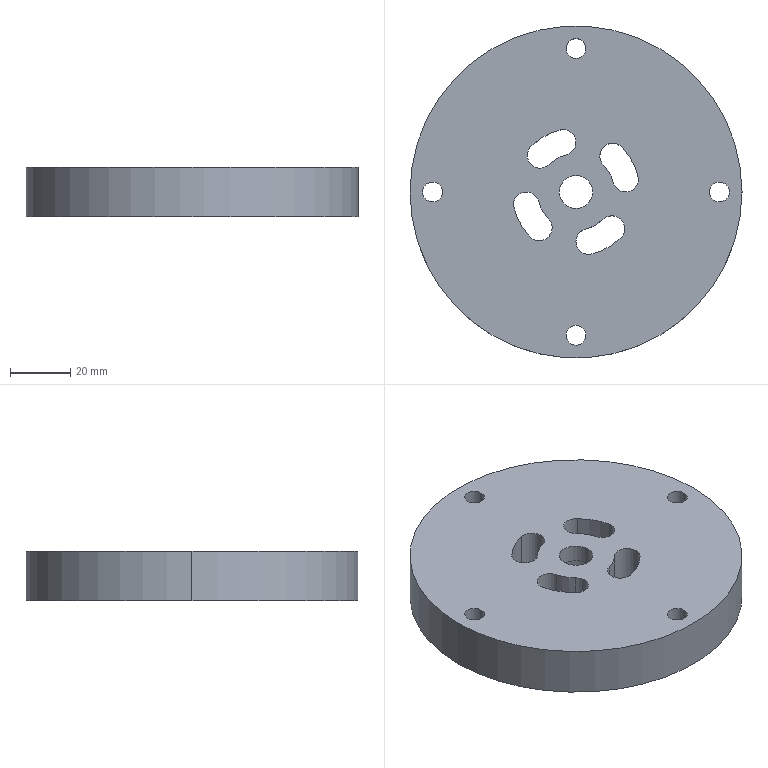Part | STEP file | 11-FG-Z01111 | 1 solid | 49 faces | box 110 x 110 x 16.5 mm | volume 141002 mm3 | cylinder 42 | plane 7 | commonest cylinder face diameters 8.5 x12 11 x10 6.6 x8 25.5 x4 42.474 x4 18 x2
STEP:
#1=CARTESIAN_POINT('',(5.5,47.5,6.4));
#2=VERTEX_POINT('',#1);
#3=CARTESIAN_POINT('',(-5.5,47.5,6.4));
#4=VERTEX_POINT('',#3);
#5=CARTESIAN_POINT('',(0.,47.5,6.4));
#6=DIRECTION('',(0.,0.,-1.));
#7=DIRECTION('',(-1.,0.,0.));
#8=AXIS2_PLACEMENT_3D('',#5,#6,#7);
#9=CIRCLE('',#8,5.5);
#10=EDGE_CURVE('',#2,#4,#9,.T.);
#11=ORIENTED_EDGE('',*,*,#10,.F.);
#12=CARTESIAN_POINT('',(5.5,47.5,0.));
#13=VERTEX_POINT('',#12);
#14=CARTESIAN_POINT('',(5.5,47.5,0.));
#15=DIRECTION('',(0.,0.,-1.));
#16=VECTOR('',#15,1000.);
#17=LINE('',#14,#16);
#18=EDGE_CURVE('',#2,#13,#17,.T.);
#19=ORIENTED_EDGE('',*,*,#18,.T.);
#20=CARTESIAN_POINT('',(-5.5,47.5,0.));
#21=VERTEX_POINT('',#20);
#22=CARTESIAN_POINT('',(0.,47.5,0.));
#23=DIRECTION('',(0.,0.,-1.));
#24=DIRECTION('',(-1.,0.,0.));
#25=AXIS2_PLACEMENT_3D('',#22,#23,#24);
#26=CIRCLE('',#25,5.5);
#27=EDGE_CURVE('',#13,#21,#26,.T.);
#28=ORIENTED_EDGE('',*,*,#27,.T.);
#29=CARTESIAN_POINT('',(-5.5,47.5,0.));
#30=DIRECTION('',(0.,0.,-1.));
#31=VECTOR('',#30,1000.);
#32=LINE('',#29,#31);
#33=EDGE_CURVE('',#4,#21,#32,.T.);
#34=ORIENTED_EDGE('',*,*,#33,.F.);
#35=EDGE_LOOP('',(#11,#19,#28,#34));
#36=FACE_OUTER_BOUND('',#35,.T.);
#37=CARTESIAN_POINT('',(0.,47.5,0.));
#38=DIRECTION('',(0.,0.,-1.));
#39=DIRECTION('',(-1.,0.,0.));
#40=AXIS2_PLACEMENT_3D('',#37,#38,#39);
#41=CYLINDRICAL_SURFACE('',#40,5.5);
#42=ADVANCED_FACE('',(#36),#41,.F.);
#43=CARTESIAN_POINT('',(-3.3,47.5,16.5));
#44=VERTEX_POINT('',#43);
#45=CARTESIAN_POINT('',(3.3,47.5,16.5));
#46=VERTEX_POINT('',#45);
#47=CARTESIAN_POINT('',(0.,47.5,16.5));
#48=DIRECTION('',(0.,0.,1.));
#49=DIRECTION('',(1.,0.,0.));
#50=AXIS2_PLACEMENT_3D('',#47,#48,#49);
#51=CIRCLE('',#50,3.3);
#52=EDGE_CURVE('',#44,#46,#51,.T.);
#53=ORIENTED_EDGE('',*,*,#52,.T.);
#54=CARTESIAN_POINT('',(3.3,47.5,6.4));
#55=VERTEX_POINT('',#54);
#56=CARTESIAN_POINT('',(3.3,47.5,0.));
#57=DIRECTION('',(0.,0.,-1.));
#58=VECTOR('',#57,1000.);
#59=LINE('',#56,#58);
#60=EDGE_CURVE('',#46,#55,#59,.T.);
#61=ORIENTED_EDGE('',*,*,#60,.T.);
#62=CARTESIAN_POINT('',(-3.3,47.5,6.4));
#63=VERTEX_POINT('',#62);
#64=CARTESIAN_POINT('',(0.,47.5,6.4));
#65=DIRECTION('',(0.,0.,-1.));
#66=DIRECTION('',(-1.,0.,0.));
#67=AXIS2_PLACEMENT_3D('',#64,#65,#66);
#68=CIRCLE('',#67,3.3);
#69=EDGE_CURVE('',#55,#63,#68,.T.);
#70=ORIENTED_EDGE('',*,*,#69,.T.);
#71=CARTESIAN_POINT('',(-3.3,47.5,0.));
#72=DIRECTION('',(0.,0.,-1.));
#73=VECTOR('',#72,1000.);
#74=LINE('',#71,#73);
#75=EDGE_CURVE('',#44,#63,#74,.T.);
#76=ORIENTED_EDGE('',*,*,#75,.F.);
#77=EDGE_LOOP('',(#53,#61,#70,#76));
#78=FACE_OUTER_BOUND('',#77,.T.);
#79=CARTESIAN_POINT('',(0.,47.5,0.));
#80=DIRECTION('',(0.,0.,-1.));
#81=DIRECTION('',(-1.,0.,0.));
#82=AXIS2_PLACEMENT_3D('',#79,#80,#81);
#83=CYLINDRICAL_SURFACE('',#82,3.3);
#84=ADVANCED_FACE('',(#78),#83,.F.);
#85=CARTESIAN_POINT('',(53.,0.,6.4));
#86=VERTEX_POINT('',#85);
#87=CARTESIAN_POINT('',(42.,0.,6.4));
#88=VERTEX_POINT('',#87);
#89=CARTESIAN_POINT('',(47.5,0.,6.4));
#90=DIRECTION('',(0.,0.,-1.));
#91=DIRECTION('',(-1.,0.,0.));
#92=AXIS2_PLACEMENT_3D('',#89,#90,#91);
#93=CIRCLE('',#92,5.5);
#94=EDGE_CURVE('',#86,#88,#93,.T.);
#95=ORIENTED_EDGE('',*,*,#94,.F.);
#96=CARTESIAN_POINT('',(53.,0.,0.));
#97=VERTEX_POINT('',#96);
#98=CARTESIAN_POINT('',(53.,0.,0.));
#99=DIRECTION('',(0.,0.,-1.));
#100=VECTOR('',#99,1000.);
#101=LINE('',#98,#100);
#102=EDGE_CURVE('',#86,#97,#101,.T.);
#103=ORIENTED_EDGE('',*,*,#102,.T.);
#104=CARTESIAN_POINT('',(42.,0.,0.));
#105=VERTEX_POINT('',#104);
#106=CARTESIAN_POINT('',(47.5,0.,0.));
#107=DIRECTION('',(0.,0.,-1.));
#108=DIRECTION('',(-1.,0.,0.));
#109=AXIS2_PLACEMENT_3D('',#106,#107,#108);
#110=CIRCLE('',#109,5.5);
#111=EDGE_CURVE('',#97,#105,#110,.T.);
#112=ORIENTED_EDGE('',*,*,#111,.T.);
#113=CARTESIAN_POINT('',(42.,0.,0.));
#114=DIRECTION('',(0.,0.,-1.));
#115=VECTOR('',#114,1000.);
#116=LINE('',#113,#115);
#117=EDGE_CURVE('',#88,#105,#116,.T.);
#118=ORIENTED_EDGE('',*,*,#117,.F.);
#119=EDGE_LOOP('',(#95,#103,#112,#118));
#120=FACE_OUTER_BOUND('',#119,.T.);
#121=CARTESIAN_POINT('',(47.5,0.,0.));
#122=DIRECTION('',(0.,0.,-1.));
#123=DIRECTION('',(-1.,0.,0.));
#124=AXIS2_PLACEMENT_3D('',#121,#122,#123);
#125=CYLINDRICAL_SURFACE('',#124,5.5);
#126=ADVANCED_FACE('',(#120),#125,.F.);
#127=CARTESIAN_POINT('',(44.2,0.,16.5));
#128=VERTEX_POINT('',#127);
#129=CARTESIAN_POINT('',(50.8,0.,16.5));
#130=VERTEX_POINT('',#129);
#131=CARTESIAN_POINT('',(47.5,0.,16.5));
#132=DIRECTION('',(0.,0.,1.));
#133=DIRECTION('',(1.,0.,0.));
#134=AXIS2_PLACEMENT_3D('',#131,#132,#133);
#135=CIRCLE('',#134,3.3);
#136=EDGE_CURVE('',#128,#130,#135,.T.);
#137=ORIENTED_EDGE('',*,*,#136,.T.);
#138=CARTESIAN_POINT('',(50.8,0.,6.4));
#139=VERTEX_POINT('',#138);
#140=CARTESIAN_POINT('',(50.8,0.,0.));
#141=DIRECTION('',(0.,0.,-1.));
#142=VECTOR('',#141,1000.);
#143=LINE('',#140,#142);
#144=EDGE_CURVE('',#130,#139,#143,.T.);
#145=ORIENTED_EDGE('',*,*,#144,.T.);
#146=CARTESIAN_POINT('',(44.2,0.,6.4));
#147=VERTEX_POINT('',#146);
#148=CARTESIAN_POINT('',(47.5,0.,6.4));
#149=DIRECTION('',(0.,0.,-1.));
#150=DIRECTION('',(-1.,0.,0.));
#151=AXIS2_PLACEMENT_3D('',#148,#149,#150);
#152=CIRCLE('',#151,3.3);
#153=EDGE_CURVE('',#139,#147,#152,.T.);
#154=ORIENTED_EDGE('',*,*,#153,.T.);
#155=CARTESIAN_POINT('',(44.2,0.,0.));
#156=DIRECTION('',(0.,0.,-1.));
#157=VECTOR('',#156,1000.);
#158=LINE('',#155,#157);
#159=EDGE_CURVE('',#128,#147,#158,.T.);
#160=ORIENTED_EDGE('',*,*,#159,.F.);
#161=EDGE_LOOP('',(#137,#145,#154,#160));
#162=FACE_OUTER_BOUND('',#161,.T.);
#163=CARTESIAN_POINT('',(47.5,0.,0.));
#164=DIRECTION('',(0.,0.,-1.));
#165=DIRECTION('',(-1.,0.,0.));
#166=AXIS2_PLACEMENT_3D('',#163,#164,#165);
#167=CYLINDRICAL_SURFACE('',#166,3.3);
#168=ADVANCED_FACE('',(#162),#167,.F.);
#169=CARTESIAN_POINT('',(5.5,-47.5,6.4));
#170=VERTEX_POINT('',#169);
#171=CARTESIAN_POINT('',(-5.5,-47.5,6.4));
#172=VERTEX_POINT('',#171);
#173=CARTESIAN_POINT('',(0.,-47.5,6.4));
#174=DIRECTION('',(0.,0.,-1.));
#175=DIRECTION('',(-1.,0.,0.));
#176=AXIS2_PLACEMENT_3D('',#173,#174,#175);
#177=CIRCLE('',#176,5.5);
#178=EDGE_CURVE('',#170,#172,#177,.T.);
#179=ORIENTED_EDGE('',*,*,#178,.F.);
#180=CARTESIAN_POINT('',(5.5,-47.5,0.));
#181=VERTEX_POINT('',#180);
#182=CARTESIAN_POINT('',(5.5,-47.5,0.));
#183=DIRECTION('',(0.,0.,-1.));
#184=VECTOR('',#183,1000.);
#185=LINE('',#182,#184);
#186=EDGE_CURVE('',#170,#181,#185,.T.);
#187=ORIENTED_EDGE('',*,*,#186,.T.);
#188=CARTESIAN_POINT('',(-5.5,-47.5,0.));
#189=VERTEX_POINT('',#188);
#190=CARTESIAN_POINT('',(0.,-47.5,0.));
#191=DIRECTION('',(0.,0.,-1.));
#192=DIRECTION('',(-1.,0.,0.));
#193=AXIS2_PLACEMENT_3D('',#190,#191,#192);
#194=CIRCLE('',#193,5.5);
#195=EDGE_CURVE('',#181,#189,#194,.T.);
#196=ORIENTED_EDGE('',*,*,#195,.T.);
#197=CARTESIAN_POINT('',(-5.5,-47.5,0.));
#198=DIRECTION('',(0.,0.,-1.));
#199=VECTOR('',#198,1000.);
#200=LINE('',#197,#199);
#201=EDGE_CURVE('',#172,#189,#200,.T.);
#202=ORIENTED_EDGE('',*,*,#201,.F.);
#203=EDGE_LOOP('',(#179,#187,#196,#202));
#204=FACE_OUTER_BOUND('',#203,.T.);
#205=CARTESIAN_POINT('',(0.,-47.5,0.));
#206=DIRECTION('',(0.,0.,-1.));
#207=DIRECTION('',(-1.,0.,0.));
#208=AXIS2_PLACEMENT_3D('',#205,#206,#207);
#209=CYLINDRICAL_SURFACE('',#208,5.5);
#210=ADVANCED_FACE('',(#204),#209,.F.);
#211=CARTESIAN_POINT('',(-3.3,-47.5,16.5));
#212=VERTEX_POINT('',#211);
#213=CARTESIAN_POINT('',(3.3,-47.5,16.5));
#214=VERTEX_POINT('',#213);
#215=CARTESIAN_POINT('',(0.,-47.5,16.5));
#216=DIRECTION('',(0.,0.,1.));
#217=DIRECTION('',(1.,0.,0.));
#218=AXIS2_PLACEMENT_3D('',#215,#216,#217);
#219=CIRCLE('',#218,3.3);
#220=EDGE_CURVE('',#212,#214,#219,.T.);
#221=ORIENTED_EDGE('',*,*,#220,.T.);
#222=CARTESIAN_POINT('',(3.3,-47.5,6.4));
#223=VERTEX_POINT('',#222);
#224=CARTESIAN_POINT('',(3.3,-47.5,0.));
#225=DIRECTION('',(0.,0.,-1.));
#226=VECTOR('',#225,1000.);
#227=LINE('',#224,#226);
#228=EDGE_CURVE('',#214,#223,#227,.T.);
#229=ORIENTED_EDGE('',*,*,#228,.T.);
#230=CARTESIAN_POINT('',(-3.3,-47.5,6.4));
#231=VERTEX_POINT('',#230);
#232=CARTESIAN_POINT('',(0.,-47.5,6.4));
#233=DIRECTION('',(0.,0.,-1.));
#234=DIRECTION('',(-1.,0.,0.));
#235=AXIS2_PLACEMENT_3D('',#232,#233,#234);
#236=CIRCLE('',#235,3.3);
#237=EDGE_CURVE('',#223,#231,#236,.T.);
#238=ORIENTED_EDGE('',*,*,#237,.T.);
#239=CARTESIAN_POINT('',(-3.3,-47.5,0.));
#240=DIRECTION('',(0.,0.,-1.));
#241=VECTOR('',#240,1000.);
#242=LINE('',#239,#241);
#243=EDGE_CURVE('',#212,#231,#242,.T.);
#244=ORIENTED_EDGE('',*,*,#243,.F.);
#245=EDGE_LOOP('',(#221,#229,#238,#244));
#246=FACE_OUTER_BOUND('',#245,.T.);
#247=CARTESIAN_POINT('',(0.,-47.5,0.));
#248=DIRECTION('',(0.,0.,-1.));
#249=DIRECTION('',(-1.,0.,0.));
#250=AXIS2_PLACEMENT_3D('',#247,#248,#249);
#251=CYLINDRICAL_SURFACE('',#250,3.3);
#252=ADVANCED_FACE('',(#246),#251,.F.);
#253=CARTESIAN_POINT('',(-42.,0.,6.4));
#254=VERTEX_POINT('',#253);
#255=CARTESIAN_POINT('',(-53.,0.,6.4));
#256=VERTEX_POINT('',#255);
#257=CARTESIAN_POINT('',(-47.5,0.,6.4));
#258=DIRECTION('',(0.,0.,-1.));
#259=DIRECTION('',(-1.,0.,0.));
#260=AXIS2_PLACEMENT_3D('',#257,#258,#259);
#261=CIRCLE('',#260,5.5);
#262=EDGE_CURVE('',#254,#256,#261,.T.);
#263=ORIENTED_EDGE('',*,*,#262,.F.);
#264=CARTESIAN_POINT('',(-42.,0.,0.));
#265=VERTEX_POINT('',#264);
#266=CARTESIAN_POINT('',(-42.,0.,0.));
#267=DIRECTION('',(0.,0.,-1.));
#268=VECTOR('',#267,1000.);
#269=LINE('',#266,#268);
#270=EDGE_CURVE('',#254,#265,#269,.T.);
#271=ORIENTED_EDGE('',*,*,#270,.T.);
#272=CARTESIAN_POINT('',(-53.,0.,0.));
#273=VERTEX_POINT('',#272);
#274=CARTESIAN_POINT('',(-47.5,0.,0.));
#275=DIRECTION('',(0.,0.,-1.));
#276=DIRECTION('',(-1.,0.,0.));
#277=AXIS2_PLACEMENT_3D('',#274,#275,#276);
#278=CIRCLE('',#277,5.5);
#279=EDGE_CURVE('',#265,#273,#278,.T.);
#280=ORIENTED_EDGE('',*,*,#279,.T.);
#281=CARTESIAN_POINT('',(-53.,0.,0.));
#282=DIRECTION('',(0.,0.,-1.));
#283=VECTOR('',#282,1000.);
#284=LINE('',#281,#283);
#285=EDGE_CURVE('',#256,#273,#284,.T.);
#286=ORIENTED_EDGE('',*,*,#285,.F.);
#287=EDGE_LOOP('',(#263,#271,#280,#286));
#288=FACE_OUTER_BOUND('',#287,.T.);
#289=CARTESIAN_POINT('',(-47.5,0.,0.));
#290=DIRECTION('',(0.,0.,-1.));
#291=DIRECTION('',(-1.,0.,0.));
#292=AXIS2_PLACEMENT_3D('',#289,#290,#291);
#293=CYLINDRICAL_SURFACE('',#292,5.5);
#294=ADVANCED_FACE('',(#288),#293,.F.);
#295=CARTESIAN_POINT('',(-50.8,0.,16.5));
#296=VERTEX_POINT('',#295);
#297=CARTESIAN_POINT('',(-44.2,0.,16.5));
#298=VERTEX_POINT('',#297);
#299=CARTESIAN_POINT('',(-47.5,0.,16.5));
#300=DIRECTION('',(0.,0.,1.));
#301=DIRECTION('',(1.,0.,0.));
#302=AXIS2_PLACEMENT_3D('',#299,#300,#301);
#303=CIRCLE('',#302,3.3);
#304=EDGE_CURVE('',#296,#298,#303,.T.);
#305=ORIENTED_EDGE('',*,*,#304,.T.);
#306=CARTESIAN_POINT('',(-44.2,0.,6.4));
#307=VERTEX_POINT('',#306);
#308=CARTESIAN_POINT('',(-44.2,0.,0.));
#309=DIRECTION('',(0.,0.,-1.));
#310=VECTOR('',#309,1000.);
#311=LINE('',#308,#310);
#312=EDGE_CURVE('',#298,#307,#311,.T.);
#313=ORIENTED_EDGE('',*,*,#312,.T.);
#314=CARTESIAN_POINT('',(-50.8,0.,6.4));
#315=VERTEX_POINT('',#314);
#316=CARTESIAN_POINT('',(-47.5,0.,6.4));
#317=DIRECTION('',(0.,0.,-1.));
#318=DIRECTION('',(-1.,0.,0.));
#319=AXIS2_PLACEMENT_3D('',#316,#317,#318);
#320=CIRCLE('',#319,3.3);
#321=EDGE_CURVE('',#307,#315,#320,.T.);
#322=ORIENTED_EDGE('',*,*,#321,.T.);
#323=CARTESIAN_POINT('',(-50.8,0.,0.));
#324=DIRECTION('',(0.,0.,-1.));
#325=VECTOR('',#324,1000.);
#326=LINE('',#323,#325);
#327=EDGE_CURVE('',#296,#315,#326,.T.);
#328=ORIENTED_EDGE('',*,*,#327,.F.);
#329=EDGE_LOOP('',(#305,#313,#322,#328));
#330=FACE_OUTER_BOUND('',#329,.T.);
#331=CARTESIAN_POINT('',(-47.5,0.,0.));
#332=DIRECTION('',(0.,0.,-1.));
#333=DIRECTION('',(-1.,0.,0.));
#334=AXIS2_PLACEMENT_3D('',#331,#332,#333);
#335=CYLINDRICAL_SURFACE('',#334,3.3);
#336=ADVANCED_FACE('',(#330),#335,.F.);
#337=CARTESIAN_POINT('',(15.416,14.606,16.5));
#338=VERTEX_POINT('',#337);
#339=CARTESIAN_POINT('',(7.885,11.906,16.5));
#340=VERTEX_POINT('',#339);
#341=CARTESIAN_POINT('',(12.135,11.906,16.5));
#342=DIRECTION('',(0.,0.,1.));
#343=DIRECTION('',(1.,0.,0.));
#344=AXIS2_PLACEMENT_3D('',#341,#342,#343);
#345=CIRCLE('',#344,4.25);
#346=EDGE_CURVE('',#338,#340,#345,.T.);
#347=ORIENTED_EDGE('',*,*,#346,.T.);
#348=CARTESIAN_POINT('',(7.885,11.906,0.));
#349=VERTEX_POINT('',#348);
#350=CARTESIAN_POINT('',(7.885,11.906,20.));
#351=DIRECTION('',(0.,0.,-1.));
#352=VECTOR('',#351,1000.);
#353=LINE('',#350,#352);
#354=EDGE_CURVE('',#340,#349,#353,.T.);
#355=ORIENTED_EDGE('',*,*,#354,.T.);
#356=CARTESIAN_POINT('',(15.416,14.606,0.));
#357=VERTEX_POINT('',#356);
#358=CARTESIAN_POINT('',(12.135,11.906,0.));
#359=DIRECTION('',(0.,0.,-1.));
#360=DIRECTION('',(1.,0.,0.));
#361=AXIS2_PLACEMENT_3D('',#358,#359,#360);
#362=CIRCLE('',#361,4.25);
#363=EDGE_CURVE('',#349,#357,#362,.T.);
#364=ORIENTED_EDGE('',*,*,#363,.T.);
#365=CARTESIAN_POINT('',(15.416,14.606,20.));
#366=DIRECTION('',(0.,0.,-1.));
#367=VECTOR('',#366,1000.);
#368=LINE('',#365,#367);
#369=EDGE_CURVE('',#338,#357,#368,.T.);
#370=ORIENTED_EDGE('',*,*,#369,.F.);
#371=EDGE_LOOP('',(#347,#355,#364,#370));
#372=FACE_OUTER_BOUND('',#371,.T.);
#373=CARTESIAN_POINT('',(12.135,11.906,20.));
#374=DIRECTION('',(0.,0.,-1.));
#375=DIRECTION('',(-1.,0.,0.));
#376=AXIS2_PLACEMENT_3D('',#373,#374,#375);
#377=CYLINDRICAL_SURFACE('',#376,4.25);
#378=ADVANCED_FACE('',(#372),#377,.F.);
#379=CARTESIAN_POINT('',(-14.606,15.416,16.5));
#380=VERTEX_POINT('',#379);
#381=CARTESIAN_POINT('',(-16.156,12.135,16.5));
#382=VERTEX_POINT('',#381);
#383=CARTESIAN_POINT('',(-11.906,12.135,16.5));
#384=DIRECTION('',(0.,0.,1.));
#385=DIRECTION('',(1.,0.,0.));
#386=AXIS2_PLACEMENT_3D('',#383,#384,#385);
#387=CIRCLE('',#386,4.25);
#388=EDGE_CURVE('',#380,#382,#387,.T.);
#389=ORIENTED_EDGE('',*,*,#388,.T.);
#390=CARTESIAN_POINT('',(-16.156,12.135,0.));
#391=VERTEX_POINT('',#390);
#392=CARTESIAN_POINT('',(-16.156,12.135,20.));
#393=DIRECTION('',(0.,0.,-1.));
#394=VECTOR('',#393,1000.);
#395=LINE('',#392,#394);
#396=EDGE_CURVE('',#382,#391,#395,.T.);
#397=ORIENTED_EDGE('',*,*,#396,.T.);
#398=CARTESIAN_POINT('',(-14.606,15.416,0.));
#399=VERTEX_POINT('',#398);
#400=CARTESIAN_POINT('',(-11.906,12.135,0.));
#401=DIRECTION('',(0.,0.,-1.));
#402=DIRECTION('',(0.,1.,0.));
#403=AXIS2_PLACEMENT_3D('',#400,#401,#402);
#404=CIRCLE('',#403,4.25);
#405=EDGE_CURVE('',#391,#399,#404,.T.);
#406=ORIENTED_EDGE('',*,*,#405,.T.);
#407=CARTESIAN_POINT('',(-14.606,15.416,20.));
#408=DIRECTION('',(0.,0.,-1.));
#409=VECTOR('',#408,1000.);
#410=LINE('',#407,#409);
#411=EDGE_CURVE('',#380,#399,#410,.T.);
#412=ORIENTED_EDGE('',*,*,#411,.F.);
#413=EDGE_LOOP('',(#389,#397,#406,#412));
#414=FACE_OUTER_BOUND('',#413,.T.);
#415=CARTESIAN_POINT('',(-11.906,12.135,20.));
#416=DIRECTION('',(0.,0.,-1.));
#417=DIRECTION('',(-1.,0.,0.));
#418=AXIS2_PLACEMENT_3D('',#415,#416,#417);
#419=CYLINDRICAL_SURFACE('',#418,4.25);
#420=ADVANCED_FACE('',(#414),#419,.F.);
#421=CARTESIAN_POINT('',(3.182,-12.346,16.5));
#422=VERTEX_POINT('',#421);
#423=CARTESIAN_POINT('',(-0.006846,-16.462,16.5));
#424=VERTEX_POINT('',#423);
#425=CARTESIAN_POINT('',(4.243,-16.462,16.5));
#426=DIRECTION('',(0.,0.,1.));
#427=DIRECTION('',(1.,0.,0.));
#428=AXIS2_PLACEMENT_3D('',#425,#426,#427);
#429=CIRCLE('',#428,4.25);
#430=EDGE_CURVE('',#422,#424,#429,.T.);
#431=ORIENTED_EDGE('',*,*,#430,.T.);
#432=CARTESIAN_POINT('',(-0.006846,-16.462,0.));
#433=VERTEX_POINT('',#432);
#434=CARTESIAN_POINT('',(-0.006846,-16.462,20.));
#435=DIRECTION('',(0.,0.,-1.));
#436=VECTOR('',#435,1000.);
#437=LINE('',#434,#436);
#438=EDGE_CURVE('',#424,#433,#437,.T.);
#439=ORIENTED_EDGE('',*,*,#438,.T.);
#440=CARTESIAN_POINT('',(3.182,-12.346,0.));
#441=VERTEX_POINT('',#440);
#442=CARTESIAN_POINT('',(4.243,-16.462,0.));
#443=DIRECTION('',(0.,0.,-1.));
#444=DIRECTION('',(0.,-1.,0.));
#445=AXIS2_PLACEMENT_3D('',#442,#443,#444);
#446=CIRCLE('',#445,4.25);
#447=EDGE_CURVE('',#433,#441,#446,.T.);
#448=ORIENTED_EDGE('',*,*,#447,.T.);
#449=CARTESIAN_POINT('',(3.182,-12.346,20.));
#450=DIRECTION('',(0.,0.,-1.));
#451=VECTOR('',#450,1000.);
#452=LINE('',#449,#451);
#453=EDGE_CURVE('',#422,#441,#452,.T.);
#454=ORIENTED_EDGE('',*,*,#453,.F.);
#455=EDGE_LOOP('',(#431,#439,#448,#454));
#456=FACE_OUTER_BOUND('',#455,.T.);
#457=CARTESIAN_POINT('',(4.243,-16.462,20.));
#458=DIRECTION('',(0.,0.,-1.));
#459=DIRECTION('',(-1.,0.,0.));
#460=AXIS2_PLACEMENT_3D('',#457,#458,#459);
#461=CYLINDRICAL_SURFACE('',#460,4.25);
#462=ADVANCED_FACE('',(#456),#461,.F.);
#463=CARTESIAN_POINT('',(-12.346,-3.182,16.5));
#464=VERTEX_POINT('',#463);
#465=CARTESIAN_POINT('',(-20.712,-4.243,16.5));
#466=VERTEX_POINT('',#465);
#467=CARTESIAN_POINT('',(-16.462,-4.243,16.5));
#468=DIRECTION('',(0.,0.,1.));
#469=DIRECTION('',(1.,0.,0.));
#470=AXIS2_PLACEMENT_3D('',#467,#468,#469);
#471=CIRCLE('',#470,4.25);
#472=EDGE_CURVE('',#464,#466,#471,.T.);
#473=ORIENTED_EDGE('',*,*,#472,.T.);
#474=CARTESIAN_POINT('',(-20.712,-4.243,0.));
#475=VERTEX_POINT('',#474);
#476=CARTESIAN_POINT('',(-20.712,-4.243,20.));
#477=DIRECTION('',(0.,0.,-1.));
#478=VECTOR('',#477,1000.);
#479=LINE('',#476,#478);
#480=EDGE_CURVE('',#466,#475,#479,.T.);
#481=ORIENTED_EDGE('',*,*,#480,.T.);
#482=CARTESIAN_POINT('',(-12.346,-3.182,0.));
#483=VERTEX_POINT('',#482);
#484=CARTESIAN_POINT('',(-16.462,-4.243,0.));
#485=DIRECTION('',(0.,0.,-1.));
#486=DIRECTION('',(-1.,0.,0.));
#487=AXIS2_PLACEMENT_3D('',#484,#485,#486);
#488=CIRCLE('',#487,4.25);
#489=EDGE_CURVE('',#475,#483,#488,.T.);
#490=ORIENTED_EDGE('',*,*,#489,.T.);
#491=CARTESIAN_POINT('',(-12.346,-3.182,20.));
#492=DIRECTION('',(0.,0.,-1.));
#493=VECTOR('',#492,1000.);
#494=LINE('',#491,#493);
#495=EDGE_CURVE('',#464,#483,#494,.T.);
#496=ORIENTED_EDGE('',*,*,#495,.F.);
#497=EDGE_LOOP('',(#473,#481,#490,#496));
#498=FACE_OUTER_BOUND('',#497,.T.);
#499=CARTESIAN_POINT('',(-16.462,-4.243,20.));
#500=DIRECTION('',(0.,0.,-1.));
#501=DIRECTION('',(-1.,0.,0.));
#502=AXIS2_PLACEMENT_3D('',#499,#500,#501);
#503=CYLINDRICAL_SURFACE('',#502,4.25);
#504=ADVANCED_FACE('',(#498),#503,.F.);
#505=CARTESIAN_POINT('',(9.,0.,10.6));
#506=VERTEX_POINT('',#505);
#507=CARTESIAN_POINT('',(-9.,0.,10.6));
#508=VERTEX_POINT('',#507);
#509=CARTESIAN_POINT('',(0.,0.,10.6));
#510=DIRECTION('',(0.,0.,-1.));
#511=DIRECTION('',(-1.,0.,0.));
#512=AXIS2_PLACEMENT_3D('',#509,#510,#511);
#513=CIRCLE('',#512,9.);
#514=EDGE_CURVE('',#506,#508,#513,.T.);
#515=ORIENTED_EDGE('',*,*,#514,.F.);
#516=CARTESIAN_POINT('',(9.,0.,0.));
#517=VERTEX_POINT('',#516);
#518=CARTESIAN_POINT('',(9.,0.,0.));
#519=DIRECTION('',(0.,0.,-1.));
#520=VECTOR('',#519,1000.);
#521=LINE('',#518,#520);
#522=EDGE_CURVE('',#506,#517,#521,.T.);
#523=ORIENTED_EDGE('',*,*,#522,.T.);
#524=CARTESIAN_POINT('',(-9.,0.,0.));
#525=VERTEX_POINT('',#524);
#526=CARTESIAN_POINT('',(0.,0.,0.));
#527=DIRECTION('',(0.,0.,-1.));
#528=DIRECTION('',(-1.,0.,0.));
#529=AXIS2_PLACEMENT_3D('',#526,#527,#528);
#530=CIRCLE('',#529,9.);
#531=EDGE_CURVE('',#517,#525,#530,.T.);
#532=ORIENTED_EDGE('',*,*,#531,.T.);
#533=CARTESIAN_POINT('',(-9.,0.,0.));
#534=DIRECTION('',(0.,0.,-1.));
#535=VECTOR('',#534,1000.);
#536=LINE('',#533,#535);
#537=EDGE_CURVE('',#508,#525,#536,.T.);
#538=ORIENTED_EDGE('',*,*,#537,.F.);
#539=EDGE_LOOP('',(#515,#523,#532,#538));
#540=FACE_OUTER_BOUND('',#539,.T.);
#541=CARTESIAN_POINT('',(0.,0.,0.));
#542=DIRECTION('',(0.,0.,-1.));
#543=DIRECTION('',(-1.,0.,0.));
#544=AXIS2_PLACEMENT_3D('',#541,#542,#543);
#545=CYLINDRICAL_SURFACE('',#544,9.);
#546=ADVANCED_FACE('',(#540),#545,.F.);
#547=CARTESIAN_POINT('',(-5.5,0.,16.5));
#548=VERTEX_POINT('',#547);
#549=CARTESIAN_POINT('',(5.5,0.,16.5));
#550=VERTEX_POINT('',#549);
#551=CARTESIAN_POINT('',(0.,0.,16.5));
#552=DIRECTION('',(0.,0.,1.));
#553=DIRECTION('',(1.,0.,0.));
#554=AXIS2_PLACEMENT_3D('',#551,#552,#553);
#555=CIRCLE('',#554,5.5);
#556=EDGE_CURVE('',#548,#550,#555,.T.);
#557=ORIENTED_EDGE('',*,*,#556,.T.);
#558=CARTESIAN_POINT('',(5.5,0.,10.6));
#559=VERTEX_POINT('',#558);
#560=CARTESIAN_POINT('',(5.5,0.,0.));
#561=DIRECTION('',(0.,0.,-1.));
#562=VECTOR('',#561,1000.);
#563=LINE('',#560,#562);
#564=EDGE_CURVE('',#550,#559,#563,.T.);
#565=ORIENTED_EDGE('',*,*,#564,.T.);
#566=CARTESIAN_POINT('',(-5.5,0.,10.6));
#567=VERTEX_POINT('',#566);
#568=CARTESIAN_POINT('',(0.,0.,10.6));
#569=DIRECTION('',(0.,0.,-1.));
#570=DIRECTION('',(-1.,0.,0.));
#571=AXIS2_PLACEMENT_3D('',#568,#569,#570);
#572=CIRCLE('',#571,5.5);
#573=EDGE_CURVE('',#559,#567,#572,.T.);
#574=ORIENTED_EDGE('',*,*,#573,.T.);
#575=CARTESIAN_POINT('',(-5.5,0.,0.));
#576=DIRECTION('',(0.,0.,-1.));
#577=VECTOR('',#576,1000.);
#578=LINE('',#575,#577);
#579=EDGE_CURVE('',#548,#567,#578,.T.);
#580=ORIENTED_EDGE('',*,*,#579,.F.);
#581=EDGE_LOOP('',(#557,#565,#574,#580));
#582=FACE_OUTER_BOUND('',#581,.T.);
#583=CARTESIAN_POINT('',(0.,0.,0.));
#584=DIRECTION('',(0.,0.,-1.));
#585=DIRECTION('',(-1.,0.,0.));
#586=AXIS2_PLACEMENT_3D('',#583,#584,#585);
#587=CYLINDRICAL_SURFACE('',#586,5.5);
#588=ADVANCED_FACE('',(#582),#587,.F.);
#589=CARTESIAN_POINT('',(55.,0.,16.5));
#590=VERTEX_POINT('',#589);
#591=CARTESIAN_POINT('',(-55.,0.,16.5));
#592=VERTEX_POINT('',#591);
#593=CARTESIAN_POINT('',(0.,0.,16.5));
#594=DIRECTION('',(0.,0.,1.));
#595=DIRECTION('',(1.,0.,0.));
#596=AXIS2_PLACEMENT_3D('',#593,#594,#595);
#597=CIRCLE('',#596,55.);
#598=EDGE_CURVE('',#590,#592,#597,.T.);
#599=ORIENTED_EDGE('',*,*,#598,.F.);
#600=CARTESIAN_POINT('',(55.,0.,0.));
#601=VERTEX_POINT('',#600);
#602=CARTESIAN_POINT('',(55.,0.,16.5));
#603=DIRECTION('',(0.,0.,-1.));
#604=VECTOR('',#603,1000.);
#605=LINE('',#602,#604);
#606=EDGE_CURVE('',#590,#601,#605,.T.);
#607=ORIENTED_EDGE('',*,*,#606,.T.);
#608=CARTESIAN_POINT('',(-55.,0.,0.));
#609=VERTEX_POINT('',#608);
#610=CARTESIAN_POINT('',(0.,0.,0.));
#611=DIRECTION('',(0.,0.,1.));
#612=DIRECTION('',(1.,0.,0.));
#613=AXIS2_PLACEMENT_3D('',#610,#611,#612);
#614=CIRCLE('',#613,55.);
#615=EDGE_CURVE('',#601,#609,#614,.T.);
#616=ORIENTED_EDGE('',*,*,#615,.T.);
#617=CARTESIAN_POINT('',(-55.,0.,16.5));
#618=DIRECTION('',(0.,0.,-1.));
#619=VECTOR('',#618,1000.);
#620=LINE('',#617,#619);
#621=EDGE_CURVE('',#592,#609,#620,.T.);
#622=ORIENTED_EDGE('',*,*,#621,.F.);
#623=EDGE_LOOP('',(#599,#607,#616,#622));
#624=FACE_OUTER_BOUND('',#623,.T.);
#625=CARTESIAN_POINT('',(0.,0.,16.5));
#626=DIRECTION('',(0.,0.,-1.));
#627=DIRECTION('',(-1.,0.,0.));
#628=AXIS2_PLACEMENT_3D('',#625,#626,#627);
#629=CYLINDRICAL_SURFACE('',#628,55.);
#630=ADVANCED_FACE('',(#624),#629,.T.);
#631=CARTESIAN_POINT('',(0.,47.5,0.));
#632=DIRECTION('',(0.,0.,-1.));
#633=DIRECTION('',(-1.,0.,0.));
#634=AXIS2_PLACEMENT_3D('',#631,#632,#633);
#635=CIRCLE('',#634,5.5);
#636=EDGE_CURVE('',#21,#13,#635,.T.);
#637=ORIENTED_EDGE('',*,*,#636,.F.);
#638=ORIENTED_EDGE('',*,*,#27,.F.);
#639=EDGE_LOOP('',(#637,#638));
#640=FACE_BOUND('',#639,.T.);
#641=CARTESIAN_POINT('',(47.5,0.,0.));
#642=DIRECTION('',(0.,0.,-1.));
#643=DIRECTION('',(-1.,0.,0.));
#644=AXIS2_PLACEMENT_3D('',#641,#642,#643);
#645=CIRCLE('',#644,5.5);
#646=EDGE_CURVE('',#105,#97,#645,.T.);
#647=ORIENTED_EDGE('',*,*,#646,.F.);
#648=ORIENTED_EDGE('',*,*,#111,.F.);
#649=EDGE_LOOP('',(#647,#648));
#650=FACE_BOUND('',#649,.T.);
#651=CARTESIAN_POINT('',(20.654,4.941,0.));
#652=VERTEX_POINT('',#651);
#653=CARTESIAN_POINT('',(12.346,3.182,0.));
#654=VERTEX_POINT('',#653);
#655=CARTESIAN_POINT('',(16.462,4.243,0.));
#656=DIRECTION('',(0.,0.,-1.));
#657=DIRECTION('',(1.,0.,0.));
#658=AXIS2_PLACEMENT_3D('',#655,#656,#657);
#659=CIRCLE('',#658,4.25);
#660=EDGE_CURVE('',#652,#654,#659,.T.);
#661=ORIENTED_EDGE('',*,*,#660,.F.);
#662=CARTESIAN_POINT('',(0.,0.,0.));
#663=DIRECTION('',(0.,0.,-1.));
#664=DIRECTION('',(1.,0.,0.));
#665=AXIS2_PLACEMENT_3D('',#662,#663,#664);
#666=CIRCLE('',#665,21.237);
#667=EDGE_CURVE('',#357,#652,#666,.T.);
#668=ORIENTED_EDGE('',*,*,#667,.F.);
#669=ORIENTED_EDGE('',*,*,#363,.F.);
#670=CARTESIAN_POINT('',(9.101,8.929,0.));
#671=VERTEX_POINT('',#670);
#672=CARTESIAN_POINT('',(12.135,11.906,0.));
#673=DIRECTION('',(0.,0.,-1.));
#674=DIRECTION('',(1.,0.,0.));
#675=AXIS2_PLACEMENT_3D('',#672,#673,#674);
#676=CIRCLE('',#675,4.25);
#677=EDGE_CURVE('',#671,#349,#676,.T.);
#678=ORIENTED_EDGE('',*,*,#677,.F.);
#679=CARTESIAN_POINT('',(0.,0.,0.));
#680=DIRECTION('',(0.,0.,1.));
#681=DIRECTION('',(1.,0.,0.));
#682=AXIS2_PLACEMENT_3D('',#679,#680,#681);
#683=CIRCLE('',#682,12.75);
#684=EDGE_CURVE('',#654,#671,#683,.T.);
#685=ORIENTED_EDGE('',*,*,#684,.F.);
#686=EDGE_LOOP('',(#661,#668,#669,#678,#685));
#687=FACE_BOUND('',#686,.T.);
#688=CARTESIAN_POINT('',(-4.941,20.654,0.));
#689=VERTEX_POINT('',#688);
#690=CARTESIAN_POINT('',(-3.182,12.346,0.));
#691=VERTEX_POINT('',#690);
#692=CARTESIAN_POINT('',(-4.243,16.462,0.));
#693=DIRECTION('',(0.,0.,-1.));
#694=DIRECTION('',(0.,1.,0.));
#695=AXIS2_PLACEMENT_3D('',#692,#693,#694);
#696=CIRCLE('',#695,4.25);
#697=EDGE_CURVE('',#689,#691,#696,.T.);
#698=ORIENTED_EDGE('',*,*,#697,.F.);
#699=CARTESIAN_POINT('',(0.,0.,0.));
#700=DIRECTION('',(0.,0.,-1.));
#701=DIRECTION('',(0.,1.,0.));
#702=AXIS2_PLACEMENT_3D('',#699,#700,#701);
#703=CIRCLE('',#702,21.237);
#704=EDGE_CURVE('',#399,#689,#703,.T.);
#705=ORIENTED_EDGE('',*,*,#704,.F.);
#706=ORIENTED_EDGE('',*,*,#405,.F.);
#707=CARTESIAN_POINT('',(-8.929,9.101,0.));
#708=VERTEX_POINT('',#707);
#709=CARTESIAN_POINT('',(-11.906,12.135,0.));
#710=DIRECTION('',(0.,0.,-1.));
#711=DIRECTION('',(0.,1.,0.));
#712=AXIS2_PLACEMENT_3D('',#709,#710,#711);
#713=CIRCLE('',#712,4.25);
#714=EDGE_CURVE('',#708,#391,#713,.T.);
#715=ORIENTED_EDGE('',*,*,#714,.F.);
#716=CARTESIAN_POINT('',(0.,0.,0.));
#717=DIRECTION('',(0.,0.,1.));
#718=DIRECTION('',(0.,1.,0.));
#719=AXIS2_PLACEMENT_3D('',#716,#717,#718);
#720=CIRCLE('',#719,12.75);
#721=EDGE_CURVE('',#691,#708,#720,.T.);
#722=ORIENTED_EDGE('',*,*,#721,.F.);
#723=EDGE_LOOP('',(#698,#705,#706,#715,#722));
#724=FACE_BOUND('',#723,.T.);
#725=CARTESIAN_POINT('',(4.941,-20.654,0.));
#726=VERTEX_POINT('',#725);
#727=CARTESIAN_POINT('',(4.243,-16.462,0.));
#728=DIRECTION('',(0.,0.,-1.));
#729=DIRECTION('',(0.,-1.,0.));
#730=AXIS2_PLACEMENT_3D('',#727,#728,#729);
#731=CIRCLE('',#730,4.25);
#732=EDGE_CURVE('',#726,#433,#731,.T.);
#733=ORIENTED_EDGE('',*,*,#732,.F.);
#734=CARTESIAN_POINT('',(14.606,-15.416,0.));
#735=VERTEX_POINT('',#734);
#736=CARTESIAN_POINT('',(0.,0.,0.));
#737=DIRECTION('',(0.,0.,-1.));
#738=DIRECTION('',(0.,-1.,0.));
#739=AXIS2_PLACEMENT_3D('',#736,#737,#738);
#740=CIRCLE('',#739,21.237);
#741=EDGE_CURVE('',#735,#726,#740,.T.);
#742=ORIENTED_EDGE('',*,*,#741,.F.);
#743=CARTESIAN_POINT('',(8.929,-9.101,0.));
#744=VERTEX_POINT('',#743);
#745=CARTESIAN_POINT('',(11.906,-12.135,0.));
#746=DIRECTION('',(0.,0.,-1.));
#747=DIRECTION('',(0.,-1.,0.));
#748=AXIS2_PLACEMENT_3D('',#745,#746,#747);
#749=CIRCLE('',#748,4.25);
#750=EDGE_CURVE('',#744,#735,#749,.T.);
#751=ORIENTED_EDGE('',*,*,#750,.F.);
#752=CARTESIAN_POINT('',(0.,0.,0.));
#753=DIRECTION('',(0.,0.,1.));
#754=DIRECTION('',(0.,-1.,0.));
#755=AXIS2_PLACEMENT_3D('',#752,#753,#754);
#756=CIRCLE('',#755,12.75);
#757=EDGE_CURVE('',#441,#744,#756,.T.);
#758=ORIENTED_EDGE('',*,*,#757,.F.);
#759=ORIENTED_EDGE('',*,*,#447,.F.);
#760=EDGE_LOOP('',(#733,#742,#751,#758,#759));
#761=FACE_BOUND('',#760,.T.);
#762=CARTESIAN_POINT('',(-20.654,-4.941,0.));
#763=VERTEX_POINT('',#762);
#764=CARTESIAN_POINT('',(-16.462,-4.243,0.));
#765=DIRECTION('',(0.,0.,-1.));
#766=DIRECTION('',(-1.,0.,0.));
#767=AXIS2_PLACEMENT_3D('',#764,#765,#766);
#768=CIRCLE('',#767,4.25);
#769=EDGE_CURVE('',#763,#475,#768,.T.);
#770=ORIENTED_EDGE('',*,*,#769,.F.);
#771=CARTESIAN_POINT('',(-15.416,-14.606,0.));
#772=VERTEX_POINT('',#771);
#773=CARTESIAN_POINT('',(0.,0.,0.));
#774=DIRECTION('',(0.,0.,-1.));
#775=DIRECTION('',(-1.,0.,0.));
#776=AXIS2_PLACEMENT_3D('',#773,#774,#775);
#777=CIRCLE('',#776,21.237);
#778=EDGE_CURVE('',#772,#763,#777,.T.);
#779=ORIENTED_EDGE('',*,*,#778,.F.);
#780=CARTESIAN_POINT('',(-9.101,-8.929,0.));
#781=VERTEX_POINT('',#780);
#782=CARTESIAN_POINT('',(-12.135,-11.906,0.));
#783=DIRECTION('',(0.,0.,-1.));
#784=DIRECTION('',(-1.,0.,0.));
#785=AXIS2_PLACEMENT_3D('',#782,#783,#784);
#786=CIRCLE('',#785,4.25);
#787=EDGE_CURVE('',#781,#772,#786,.T.);
#788=ORIENTED_EDGE('',*,*,#787,.F.);
#789=CARTESIAN_POINT('',(0.,0.,0.));
#790=DIRECTION('',(0.,0.,1.));
#791=DIRECTION('',(-1.,0.,0.));
#792=AXIS2_PLACEMENT_3D('',#789,#790,#791);
#793=CIRCLE('',#792,12.75);
#794=EDGE_CURVE('',#483,#781,#793,.T.);
#795=ORIENTED_EDGE('',*,*,#794,.F.);
#796=ORIENTED_EDGE('',*,*,#489,.F.);
#797=EDGE_LOOP('',(#770,#779,#788,#795,#796));
#798=FACE_BOUND('',#797,.T.);
#799=CARTESIAN_POINT('',(0.,0.,0.));
#800=DIRECTION('',(0.,0.,-1.));
#801=DIRECTION('',(-1.,0.,0.));
#802=AXIS2_PLACEMENT_3D('',#799,#800,#801);
#803=CIRCLE('',#802,9.);
#804=EDGE_CURVE('',#525,#517,#803,.T.);
#805=ORIENTED_EDGE('',*,*,#804,.F.);
#806=ORIENTED_EDGE('',*,*,#531,.F.);
#807=EDGE_LOOP('',(#805,#806));
#808=FACE_BOUND('',#807,.T.);
#809=CARTESIAN_POINT('',(0.,0.,0.));
#810=DIRECTION('',(0.,0.,1.));
#811=DIRECTION('',(1.,0.,0.));
#812=AXIS2_PLACEMENT_3D('',#809,#810,#811);
#813=CIRCLE('',#812,55.);
#814=EDGE_CURVE('',#609,#601,#813,.T.);
#815=ORIENTED_EDGE('',*,*,#814,.F.);
#816=ORIENTED_EDGE('',*,*,#615,.F.);
#817=EDGE_LOOP('',(#815,#816));
#818=FACE_OUTER_BOUND('',#817,.T.);
#819=CARTESIAN_POINT('',(-47.5,0.,0.));
#820=DIRECTION('',(0.,0.,-1.));
#821=DIRECTION('',(-1.,0.,0.));
#822=AXIS2_PLACEMENT_3D('',#819,#820,#821);
#823=CIRCLE('',#822,5.5);
#824=EDGE_CURVE('',#273,#265,#823,.T.);
#825=ORIENTED_EDGE('',*,*,#824,.F.);
#826=ORIENTED_EDGE('',*,*,#279,.F.);
#827=EDGE_LOOP('',(#825,#826));
#828=FACE_BOUND('',#827,.T.);
#829=CARTESIAN_POINT('',(0.,-47.5,0.));
#830=DIRECTION('',(0.,0.,-1.));
#831=DIRECTION('',(-1.,0.,0.));
#832=AXIS2_PLACEMENT_3D('',#829,#830,#831);
#833=CIRCLE('',#832,5.5);
#834=EDGE_CURVE('',#189,#181,#833,.T.);
#835=ORIENTED_EDGE('',*,*,#834,.F.);
#836=ORIENTED_EDGE('',*,*,#195,.F.);
#837=EDGE_LOOP('',(#835,#836));
#838=FACE_BOUND('',#837,.T.);
#839=CARTESIAN_POINT('',(0.,0.,0.));
#840=DIRECTION('',(0.,0.,1.));
#841=DIRECTION('',(1.,0.,0.));
#842=AXIS2_PLACEMENT_3D('',#839,#840,#841);
#843=PLANE('',#842);
#844=ADVANCED_FACE('',(#640,#650,#687,#724,#761,#798,#808,#818,#828,#838),#843,.F.);
#845=ORIENTED_EDGE('',*,*,#606,.F.);
#846=CARTESIAN_POINT('',(0.,0.,16.5));
#847=DIRECTION('',(0.,0.,1.));
#848=DIRECTION('',(1.,0.,0.));
#849=AXIS2_PLACEMENT_3D('',#846,#847,#848);
#850=CIRCLE('',#849,55.);
#851=EDGE_CURVE('',#592,#590,#850,.T.);
#852=ORIENTED_EDGE('',*,*,#851,.F.);
#853=ORIENTED_EDGE('',*,*,#621,.T.);
#854=ORIENTED_EDGE('',*,*,#814,.T.);
#855=EDGE_LOOP('',(#845,#852,#853,#854));
#856=FACE_OUTER_BOUND('',#855,.T.);
#857=CARTESIAN_POINT('',(0.,0.,16.5));
#858=DIRECTION('',(0.,0.,-1.));
#859=DIRECTION('',(-1.,0.,0.));
#860=AXIS2_PLACEMENT_3D('',#857,#858,#859);
#861=CYLINDRICAL_SURFACE('',#860,55.);
#862=ADVANCED_FACE('',(#856),#861,.T.);
#863=ORIENTED_EDGE('',*,*,#52,.F.);
#864=CARTESIAN_POINT('',(0.,47.5,16.5));
#865=DIRECTION('',(0.,0.,1.));
#866=DIRECTION('',(1.,0.,0.));
#867=AXIS2_PLACEMENT_3D('',#864,#865,#866);
#868=CIRCLE('',#867,3.3);
#869=EDGE_CURVE('',#46,#44,#868,.T.);
#870=ORIENTED_EDGE('',*,*,#869,.F.);
#871=EDGE_LOOP('',(#863,#870));
#872=FACE_BOUND('',#871,.T.);
#873=ORIENTED_EDGE('',*,*,#136,.F.);
#874=CARTESIAN_POINT('',(47.5,0.,16.5));
#875=DIRECTION('',(0.,0.,1.));
#876=DIRECTION('',(1.,0.,0.));
#877=AXIS2_PLACEMENT_3D('',#874,#875,#876);
#878=CIRCLE('',#877,3.3);
#879=EDGE_CURVE('',#130,#128,#878,.T.);
#880=ORIENTED_EDGE('',*,*,#879,.F.);
#881=EDGE_LOOP('',(#873,#880));
#882=FACE_BOUND('',#881,.T.);
#883=ORIENTED_EDGE('',*,*,#220,.F.);
#884=CARTESIAN_POINT('',(0.,-47.5,16.5));
#885=DIRECTION('',(0.,0.,1.));
#886=DIRECTION('',(1.,0.,0.));
#887=AXIS2_PLACEMENT_3D('',#884,#885,#886);
#888=CIRCLE('',#887,3.3);
#889=EDGE_CURVE('',#214,#212,#888,.T.);
#890=ORIENTED_EDGE('',*,*,#889,.F.);
#891=EDGE_LOOP('',(#883,#890));
#892=FACE_BOUND('',#891,.T.);
#893=ORIENTED_EDGE('',*,*,#304,.F.);
#894=CARTESIAN_POINT('',(-47.5,0.,16.5));
#895=DIRECTION('',(0.,0.,1.));
#896=DIRECTION('',(1.,0.,0.));
#897=AXIS2_PLACEMENT_3D('',#894,#895,#896);
#898=CIRCLE('',#897,3.3);
#899=EDGE_CURVE('',#298,#296,#898,.T.);
#900=ORIENTED_EDGE('',*,*,#899,.F.);
#901=EDGE_LOOP('',(#893,#900));
#902=FACE_BOUND('',#901,.T.);
#903=CARTESIAN_POINT('',(20.654,4.941,16.5));
#904=VERTEX_POINT('',#903);
#905=CARTESIAN_POINT('',(0.,0.,16.5));
#906=DIRECTION('',(0.,0.,1.));
#907=DIRECTION('',(1.,0.,0.));
#908=AXIS2_PLACEMENT_3D('',#905,#906,#907);
#909=CIRCLE('',#908,21.237);
#910=EDGE_CURVE('',#904,#338,#909,.T.);
#911=ORIENTED_EDGE('',*,*,#910,.F.);
#912=CARTESIAN_POINT('',(12.346,3.182,16.5));
#913=VERTEX_POINT('',#912);
#914=CARTESIAN_POINT('',(16.462,4.243,16.5));
#915=DIRECTION('',(0.,0.,1.));
#916=DIRECTION('',(1.,0.,0.));
#917=AXIS2_PLACEMENT_3D('',#914,#915,#916);
#918=CIRCLE('',#917,4.25);
#919=EDGE_CURVE('',#913,#904,#918,.T.);
#920=ORIENTED_EDGE('',*,*,#919,.F.);
#921=CARTESIAN_POINT('',(9.101,8.929,16.5));
#922=VERTEX_POINT('',#921);
#923=CARTESIAN_POINT('',(0.,0.,16.5));
#924=DIRECTION('',(0.,0.,-1.));
#925=DIRECTION('',(1.,0.,0.));
#926=AXIS2_PLACEMENT_3D('',#923,#924,#925);
#927=CIRCLE('',#926,12.75);
#928=EDGE_CURVE('',#922,#913,#927,.T.);
#929=ORIENTED_EDGE('',*,*,#928,.F.);
#930=CARTESIAN_POINT('',(12.135,11.906,16.5));
#931=DIRECTION('',(0.,0.,1.));
#932=DIRECTION('',(1.,0.,0.));
#933=AXIS2_PLACEMENT_3D('',#930,#931,#932);
#934=CIRCLE('',#933,4.25);
#935=EDGE_CURVE('',#340,#922,#934,.T.);
#936=ORIENTED_EDGE('',*,*,#935,.F.);
#937=ORIENTED_EDGE('',*,*,#346,.F.);
#938=EDGE_LOOP('',(#911,#920,#929,#936,#937));
#939=FACE_BOUND('',#938,.T.);
#940=CARTESIAN_POINT('',(-4.941,20.654,16.5));
#941=VERTEX_POINT('',#940);
#942=CARTESIAN_POINT('',(0.,0.,16.5));
#943=DIRECTION('',(0.,0.,1.));
#944=DIRECTION('',(1.,0.,0.));
#945=AXIS2_PLACEMENT_3D('',#942,#943,#944);
#946=CIRCLE('',#945,21.237);
#947=EDGE_CURVE('',#941,#380,#946,.T.);
#948=ORIENTED_EDGE('',*,*,#947,.F.);
#949=CARTESIAN_POINT('',(-3.182,12.346,16.5));
#950=VERTEX_POINT('',#949);
#951=CARTESIAN_POINT('',(-4.243,16.462,16.5));
#952=DIRECTION('',(0.,0.,1.));
#953=DIRECTION('',(1.,0.,0.));
#954=AXIS2_PLACEMENT_3D('',#951,#952,#953);
#955=CIRCLE('',#954,4.25);
#956=EDGE_CURVE('',#950,#941,#955,.T.);
#957=ORIENTED_EDGE('',*,*,#956,.F.);
#958=CARTESIAN_POINT('',(-8.929,9.101,16.5));
#959=VERTEX_POINT('',#958);
#960=CARTESIAN_POINT('',(0.,0.,16.5));
#961=DIRECTION('',(0.,0.,-1.));
#962=DIRECTION('',(1.,0.,0.));
#963=AXIS2_PLACEMENT_3D('',#960,#961,#962);
#964=CIRCLE('',#963,12.75);
#965=EDGE_CURVE('',#959,#950,#964,.T.);
#966=ORIENTED_EDGE('',*,*,#965,.F.);
#967=CARTESIAN_POINT('',(-11.906,12.135,16.5));
#968=DIRECTION('',(0.,0.,1.));
#969=DIRECTION('',(1.,0.,0.));
#970=AXIS2_PLACEMENT_3D('',#967,#968,#969);
#971=CIRCLE('',#970,4.25);
#972=EDGE_CURVE('',#382,#959,#971,.T.);
#973=ORIENTED_EDGE('',*,*,#972,.F.);
#974=ORIENTED_EDGE('',*,*,#388,.F.);
#975=EDGE_LOOP('',(#948,#957,#966,#973,#974));
#976=FACE_BOUND('',#975,.T.);
#977=CARTESIAN_POINT('',(4.941,-20.654,16.5));
#978=VERTEX_POINT('',#977);
#979=CARTESIAN_POINT('',(14.606,-15.416,16.5));
#980=VERTEX_POINT('',#979);
#981=CARTESIAN_POINT('',(0.,0.,16.5));
#982=DIRECTION('',(0.,0.,1.));
#983=DIRECTION('',(1.,0.,0.));
#984=AXIS2_PLACEMENT_3D('',#981,#982,#983);
#985=CIRCLE('',#984,21.237);
#986=EDGE_CURVE('',#978,#980,#985,.T.);
#987=ORIENTED_EDGE('',*,*,#986,.F.);
#988=CARTESIAN_POINT('',(4.243,-16.462,16.5));
#989=DIRECTION('',(0.,0.,1.));
#990=DIRECTION('',(1.,0.,0.));
#991=AXIS2_PLACEMENT_3D('',#988,#989,#990);
#992=CIRCLE('',#991,4.25);
#993=EDGE_CURVE('',#424,#978,#992,.T.);
#994=ORIENTED_EDGE('',*,*,#993,.F.);
#995=ORIENTED_EDGE('',*,*,#430,.F.);
#996=CARTESIAN_POINT('',(8.929,-9.101,16.5));
#997=VERTEX_POINT('',#996);
#998=CARTESIAN_POINT('',(0.,0.,16.5));
#999=DIRECTION('',(0.,0.,-1.));
#1000=DIRECTION('',(1.,0.,0.));
#1001=AXIS2_PLACEMENT_3D('',#998,#999,#1000);
#1002=CIRCLE('',#1001,12.75);
#1003=EDGE_CURVE('',#997,#422,#1002,.T.);
#1004=ORIENTED_EDGE('',*,*,#1003,.F.);
#1005=CARTESIAN_POINT('',(11.906,-12.135,16.5));
#1006=DIRECTION('',(0.,0.,1.));
#1007=DIRECTION('',(1.,0.,0.));
#1008=AXIS2_PLACEMENT_3D('',#1005,#1006,#1007);
#1009=CIRCLE('',#1008,4.25);
#1010=EDGE_CURVE('',#980,#997,#1009,.T.);
#1011=ORIENTED_EDGE('',*,*,#1010,.F.);
#1012=EDGE_LOOP('',(#987,#994,#995,#1004,#1011));
#1013=FACE_BOUND('',#1012,.T.);
#1014=CARTESIAN_POINT('',(-20.654,-4.941,16.5));
#1015=VERTEX_POINT('',#1014);
#1016=CARTESIAN_POINT('',(-15.416,-14.606,16.5));
#1017=VERTEX_POINT('',#1016);
#1018=CARTESIAN_POINT('',(0.,0.,16.5));
#1019=DIRECTION('',(0.,0.,1.));
#1020=DIRECTION('',(1.,0.,0.));
#1021=AXIS2_PLACEMENT_3D('',#1018,#1019,#1020);
#1022=CIRCLE('',#1021,21.237);
#1023=EDGE_CURVE('',#1015,#1017,#1022,.T.);
#1024=ORIENTED_EDGE('',*,*,#1023,.F.);
#1025=CARTESIAN_POINT('',(-16.462,-4.243,16.5));
#1026=DIRECTION('',(0.,0.,1.));
#1027=DIRECTION('',(1.,0.,0.));
#1028=AXIS2_PLACEMENT_3D('',#1025,#1026,#1027);
#1029=CIRCLE('',#1028,4.25);
#1030=EDGE_CURVE('',#466,#1015,#1029,.T.);
#1031=ORIENTED_EDGE('',*,*,#1030,.F.);
#1032=ORIENTED_EDGE('',*,*,#472,.F.);
#1033=CARTESIAN_POINT('',(-9.101,-8.929,16.5));
#1034=VERTEX_POINT('',#1033);
#1035=CARTESIAN_POINT('',(0.,0.,16.5));
#1036=DIRECTION('',(0.,0.,-1.));
#1037=DIRECTION('',(1.,0.,0.));
#1038=AXIS2_PLACEMENT_3D('',#1035,#1036,#1037);
#1039=CIRCLE('',#1038,12.75);
#1040=EDGE_CURVE('',#1034,#464,#1039,.T.);
#1041=ORIENTED_EDGE('',*,*,#1040,.F.);
#1042=CARTESIAN_POINT('',(-12.135,-11.906,16.5));
#1043=DIRECTION('',(0.,0.,1.));
#1044=DIRECTION('',(1.,0.,0.));
#1045=AXIS2_PLACEMENT_3D('',#1042,#1043,#1044);
#1046=CIRCLE('',#1045,4.25);
#1047=EDGE_CURVE('',#1017,#1034,#1046,.T.);
#1048=ORIENTED_EDGE('',*,*,#1047,.F.);
#1049=EDGE_LOOP('',(#1024,#1031,#1032,#1041,#1048));
#1050=FACE_BOUND('',#1049,.T.);
#1051=ORIENTED_EDGE('',*,*,#556,.F.);
#1052=CARTESIAN_POINT('',(0.,0.,16.5));
#1053=DIRECTION('',(0.,0.,1.));
#1054=DIRECTION('',(1.,0.,0.));
#1055=AXIS2_PLACEMENT_3D('',#1052,#1053,#1054);
#1056=CIRCLE('',#1055,5.5);
#1057=EDGE_CURVE('',#550,#548,#1056,.T.);
#1058=ORIENTED_EDGE('',*,*,#1057,.F.);
#1059=EDGE_LOOP('',(#1051,#1058));
#1060=FACE_BOUND('',#1059,.T.);
#1061=ORIENTED_EDGE('',*,*,#851,.T.);
#1062=ORIENTED_EDGE('',*,*,#598,.T.);
#1063=EDGE_LOOP('',(#1061,#1062));
#1064=FACE_OUTER_BOUND('',#1063,.T.);
#1065=CARTESIAN_POINT('',(0.,0.,16.5));
#1066=DIRECTION('',(0.,0.,1.));
#1067=DIRECTION('',(1.,0.,0.));
#1068=AXIS2_PLACEMENT_3D('',#1065,#1066,#1067);
#1069=PLANE('',#1068);
#1070=ADVANCED_FACE('',(#872,#882,#892,#902,#939,#976,#1013,#1050,#1060,#1064),#1069,.T.);
#1071=ORIENTED_EDGE('',*,*,#564,.F.);
#1072=ORIENTED_EDGE('',*,*,#1057,.T.);
#1073=ORIENTED_EDGE('',*,*,#579,.T.);
#1074=CARTESIAN_POINT('',(0.,0.,10.6));
#1075=DIRECTION('',(0.,0.,-1.));
#1076=DIRECTION('',(-1.,0.,0.));
#1077=AXIS2_PLACEMENT_3D('',#1074,#1075,#1076);
#1078=CIRCLE('',#1077,5.5);
#1079=EDGE_CURVE('',#567,#559,#1078,.T.);
#1080=ORIENTED_EDGE('',*,*,#1079,.T.);
#1081=EDGE_LOOP('',(#1071,#1072,#1073,#1080));
#1082=FACE_OUTER_BOUND('',#1081,.T.);
#1083=CARTESIAN_POINT('',(0.,0.,0.));
#1084=DIRECTION('',(0.,0.,-1.));
#1085=DIRECTION('',(-1.,0.,0.));
#1086=AXIS2_PLACEMENT_3D('',#1083,#1084,#1085);
#1087=CYLINDRICAL_SURFACE('',#1086,5.5);
#1088=ADVANCED_FACE('',(#1082),#1087,.F.);
#1089=ORIENTED_EDGE('',*,*,#1079,.F.);
#1090=ORIENTED_EDGE('',*,*,#573,.F.);
#1091=EDGE_LOOP('',(#1089,#1090));
#1092=FACE_BOUND('',#1091,.T.);
#1093=CARTESIAN_POINT('',(0.,0.,10.6));
#1094=DIRECTION('',(0.,0.,-1.));
#1095=DIRECTION('',(-1.,0.,0.));
#1096=AXIS2_PLACEMENT_3D('',#1093,#1094,#1095);
#1097=CIRCLE('',#1096,9.);
#1098=EDGE_CURVE('',#508,#506,#1097,.T.);
#1099=ORIENTED_EDGE('',*,*,#1098,.T.);
#1100=ORIENTED_EDGE('',*,*,#514,.T.);
#1101=EDGE_LOOP('',(#1099,#1100));
#1102=FACE_OUTER_BOUND('',#1101,.T.);
#1103=CARTESIAN_POINT('',(5.5,0.,10.6));
#1104=DIRECTION('',(0.,0.,1.));
#1105=DIRECTION('',(1.,0.,0.));
#1106=AXIS2_PLACEMENT_3D('',#1103,#1104,#1105);
#1107=PLANE('',#1106);
#1108=ADVANCED_FACE('',(#1092,#1102),#1107,.F.);
#1109=ORIENTED_EDGE('',*,*,#522,.F.);
#1110=ORIENTED_EDGE('',*,*,#1098,.F.);
#1111=ORIENTED_EDGE('',*,*,#537,.T.);
#1112=ORIENTED_EDGE('',*,*,#804,.T.);
#1113=EDGE_LOOP('',(#1109,#1110,#1111,#1112));
#1114=FACE_OUTER_BOUND('',#1113,.T.);
#1115=CARTESIAN_POINT('',(0.,0.,0.));
#1116=DIRECTION('',(0.,0.,-1.));
#1117=DIRECTION('',(-1.,0.,0.));
#1118=AXIS2_PLACEMENT_3D('',#1115,#1116,#1117);
#1119=CYLINDRICAL_SURFACE('',#1118,9.);
#1120=ADVANCED_FACE('',(#1114),#1119,.F.);
#1121=ORIENTED_EDGE('',*,*,#1023,.T.);
#1122=CARTESIAN_POINT('',(-15.416,-14.606,20.));
#1123=DIRECTION('',(0.,0.,-1.));
#1124=VECTOR('',#1123,1000.);
#1125=LINE('',#1122,#1124);
#1126=EDGE_CURVE('',#1017,#772,#1125,.T.);
#1127=ORIENTED_EDGE('',*,*,#1126,.T.);
#1128=ORIENTED_EDGE('',*,*,#778,.T.);
#1129=CARTESIAN_POINT('',(-20.654,-4.941,20.));
#1130=DIRECTION('',(0.,0.,-1.));
#1131=VECTOR('',#1130,1000.);
#1132=LINE('',#1129,#1131);
#1133=EDGE_CURVE('',#1015,#763,#1132,.T.);
#1134=ORIENTED_EDGE('',*,*,#1133,.F.);
#1135=EDGE_LOOP('',(#1121,#1127,#1128,#1134));
#1136=FACE_OUTER_BOUND('',#1135,.T.);
#1137=CARTESIAN_POINT('',(0.,0.,20.));
#1138=DIRECTION('',(0.,0.,-1.));
#1139=DIRECTION('',(-1.,0.,0.));
#1140=AXIS2_PLACEMENT_3D('',#1137,#1138,#1139);
#1141=CYLINDRICAL_SURFACE('',#1140,21.237);
#1142=ADVANCED_FACE('',(#1136),#1141,.F.);
#1143=ORIENTED_EDGE('',*,*,#1047,.T.);
#1144=CARTESIAN_POINT('',(-9.101,-8.929,20.));
#1145=DIRECTION('',(0.,0.,-1.));
#1146=VECTOR('',#1145,1000.);
#1147=LINE('',#1144,#1146);
#1148=EDGE_CURVE('',#1034,#781,#1147,.T.);
#1149=ORIENTED_EDGE('',*,*,#1148,.T.);
#1150=ORIENTED_EDGE('',*,*,#787,.T.);
#1151=ORIENTED_EDGE('',*,*,#1126,.F.);
#1152=EDGE_LOOP('',(#1143,#1149,#1150,#1151));
#1153=FACE_OUTER_BOUND('',#1152,.T.);
#1154=CARTESIAN_POINT('',(-12.135,-11.906,20.));
#1155=DIRECTION('',(0.,0.,-1.));
#1156=DIRECTION('',(-1.,0.,0.));
#1157=AXIS2_PLACEMENT_3D('',#1154,#1155,#1156);
#1158=CYLINDRICAL_SURFACE('',#1157,4.25);
#1159=ADVANCED_FACE('',(#1153),#1158,.F.);
#1160=ORIENTED_EDGE('',*,*,#1040,.T.);
#1161=ORIENTED_EDGE('',*,*,#495,.T.);
#1162=ORIENTED_EDGE('',*,*,#794,.T.);
#1163=ORIENTED_EDGE('',*,*,#1148,.F.);
#1164=EDGE_LOOP('',(#1160,#1161,#1162,#1163));
#1165=FACE_OUTER_BOUND('',#1164,.T.);
#1166=CARTESIAN_POINT('',(0.,0.,20.));
#1167=DIRECTION('',(0.,0.,-1.));
#1168=DIRECTION('',(-1.,0.,0.));
#1169=AXIS2_PLACEMENT_3D('',#1166,#1167,#1168);
#1170=CYLINDRICAL_SURFACE('',#1169,12.75);
#1171=ADVANCED_FACE('',(#1165),#1170,.T.);
#1172=ORIENTED_EDGE('',*,*,#480,.F.);
#1173=ORIENTED_EDGE('',*,*,#1030,.T.);
#1174=ORIENTED_EDGE('',*,*,#1133,.T.);
#1175=ORIENTED_EDGE('',*,*,#769,.T.);
#1176=EDGE_LOOP('',(#1172,#1173,#1174,#1175));
#1177=FACE_OUTER_BOUND('',#1176,.T.);
#1178=CARTESIAN_POINT('',(-16.462,-4.243,20.));
#1179=DIRECTION('',(0.,0.,-1.));
#1180=DIRECTION('',(-1.,0.,0.));
#1181=AXIS2_PLACEMENT_3D('',#1178,#1179,#1180);
#1182=CYLINDRICAL_SURFACE('',#1181,4.25);
#1183=ADVANCED_FACE('',(#1177),#1182,.F.);
#1184=ORIENTED_EDGE('',*,*,#986,.T.);
#1185=CARTESIAN_POINT('',(14.606,-15.416,20.));
#1186=DIRECTION('',(0.,0.,-1.));
#1187=VECTOR('',#1186,1000.);
#1188=LINE('',#1185,#1187);
#1189=EDGE_CURVE('',#980,#735,#1188,.T.);
#1190=ORIENTED_EDGE('',*,*,#1189,.T.);
#1191=ORIENTED_EDGE('',*,*,#741,.T.);
#1192=CARTESIAN_POINT('',(4.941,-20.654,20.));
#1193=DIRECTION('',(0.,0.,-1.));
#1194=VECTOR('',#1193,1000.);
#1195=LINE('',#1192,#1194);
#1196=EDGE_CURVE('',#978,#726,#1195,.T.);
#1197=ORIENTED_EDGE('',*,*,#1196,.F.);
#1198=EDGE_LOOP('',(#1184,#1190,#1191,#1197));
#1199=FACE_OUTER_BOUND('',#1198,.T.);
#1200=CARTESIAN_POINT('',(0.,0.,20.));
#1201=DIRECTION('',(0.,0.,-1.));
#1202=DIRECTION('',(-1.,0.,0.));
#1203=AXIS2_PLACEMENT_3D('',#1200,#1201,#1202);
#1204=CYLINDRICAL_SURFACE('',#1203,21.237);
#1205=ADVANCED_FACE('',(#1199),#1204,.F.);
#1206=ORIENTED_EDGE('',*,*,#1010,.T.);
#1207=CARTESIAN_POINT('',(8.929,-9.101,20.));
#1208=DIRECTION('',(0.,0.,-1.));
#1209=VECTOR('',#1208,1000.);
#1210=LINE('',#1207,#1209);
#1211=EDGE_CURVE('',#997,#744,#1210,.T.);
#1212=ORIENTED_EDGE('',*,*,#1211,.T.);
#1213=ORIENTED_EDGE('',*,*,#750,.T.);
#1214=ORIENTED_EDGE('',*,*,#1189,.F.);
#1215=EDGE_LOOP('',(#1206,#1212,#1213,#1214));
#1216=FACE_OUTER_BOUND('',#1215,.T.);
#1217=CARTESIAN_POINT('',(11.906,-12.135,20.));
#1218=DIRECTION('',(0.,0.,-1.));
#1219=DIRECTION('',(-1.,0.,0.));
#1220=AXIS2_PLACEMENT_3D('',#1217,#1218,#1219);
#1221=CYLINDRICAL_SURFACE('',#1220,4.25);
#1222=ADVANCED_FACE('',(#1216),#1221,.F.);
#1223=ORIENTED_EDGE('',*,*,#1003,.T.);
#1224=ORIENTED_EDGE('',*,*,#453,.T.);
#1225=ORIENTED_EDGE('',*,*,#757,.T.);
#1226=ORIENTED_EDGE('',*,*,#1211,.F.);
#1227=EDGE_LOOP('',(#1223,#1224,#1225,#1226));
#1228=FACE_OUTER_BOUND('',#1227,.T.);
#1229=CARTESIAN_POINT('',(0.,0.,20.));
#1230=DIRECTION('',(0.,0.,-1.));
#1231=DIRECTION('',(-1.,0.,0.));
#1232=AXIS2_PLACEMENT_3D('',#1229,#1230,#1231);
#1233=CYLINDRICAL_SURFACE('',#1232,12.75);
#1234=ADVANCED_FACE('',(#1228),#1233,.T.);
#1235=ORIENTED_EDGE('',*,*,#438,.F.);
#1236=ORIENTED_EDGE('',*,*,#993,.T.);
#1237=ORIENTED_EDGE('',*,*,#1196,.T.);
#1238=ORIENTED_EDGE('',*,*,#732,.T.);
#1239=EDGE_LOOP('',(#1235,#1236,#1237,#1238));
#1240=FACE_OUTER_BOUND('',#1239,.T.);
#1241=CARTESIAN_POINT('',(4.243,-16.462,20.));
#1242=DIRECTION('',(0.,0.,-1.));
#1243=DIRECTION('',(-1.,0.,0.));
#1244=AXIS2_PLACEMENT_3D('',#1241,#1242,#1243);
#1245=CYLINDRICAL_SURFACE('',#1244,4.25);
#1246=ADVANCED_FACE('',(#1240),#1245,.F.);
#1247=ORIENTED_EDGE('',*,*,#947,.T.);
#1248=ORIENTED_EDGE('',*,*,#411,.T.);
#1249=ORIENTED_EDGE('',*,*,#704,.T.);
#1250=CARTESIAN_POINT('',(-4.941,20.654,20.));
#1251=DIRECTION('',(0.,0.,-1.));
#1252=VECTOR('',#1251,1000.);
#1253=LINE('',#1250,#1252);
#1254=EDGE_CURVE('',#941,#689,#1253,.T.);
#1255=ORIENTED_EDGE('',*,*,#1254,.F.);
#1256=EDGE_LOOP('',(#1247,#1248,#1249,#1255));
#1257=FACE_OUTER_BOUND('',#1256,.T.);
#1258=CARTESIAN_POINT('',(0.,0.,20.));
#1259=DIRECTION('',(0.,0.,-1.));
#1260=DIRECTION('',(-1.,0.,0.));
#1261=AXIS2_PLACEMENT_3D('',#1258,#1259,#1260);
#1262=CYLINDRICAL_SURFACE('',#1261,21.237);
#1263=ADVANCED_FACE('',(#1257),#1262,.F.);
#1264=ORIENTED_EDGE('',*,*,#396,.F.);
#1265=ORIENTED_EDGE('',*,*,#972,.T.);
#1266=CARTESIAN_POINT('',(-8.929,9.101,20.));
#1267=DIRECTION('',(0.,0.,-1.));
#1268=VECTOR('',#1267,1000.);
#1269=LINE('',#1266,#1268);
#1270=EDGE_CURVE('',#959,#708,#1269,.T.);
#1271=ORIENTED_EDGE('',*,*,#1270,.T.);
#1272=ORIENTED_EDGE('',*,*,#714,.T.);
#1273=EDGE_LOOP('',(#1264,#1265,#1271,#1272));
#1274=FACE_OUTER_BOUND('',#1273,.T.);
#1275=CARTESIAN_POINT('',(-11.906,12.135,20.));
#1276=DIRECTION('',(0.,0.,-1.));
#1277=DIRECTION('',(-1.,0.,0.));
#1278=AXIS2_PLACEMENT_3D('',#1275,#1276,#1277);
#1279=CYLINDRICAL_SURFACE('',#1278,4.25);
#1280=ADVANCED_FACE('',(#1274),#1279,.F.);
#1281=ORIENTED_EDGE('',*,*,#965,.T.);
#1282=CARTESIAN_POINT('',(-3.182,12.346,20.));
#1283=DIRECTION('',(0.,0.,-1.));
#1284=VECTOR('',#1283,1000.);
#1285=LINE('',#1282,#1284);
#1286=EDGE_CURVE('',#950,#691,#1285,.T.);
#1287=ORIENTED_EDGE('',*,*,#1286,.T.);
#1288=ORIENTED_EDGE('',*,*,#721,.T.);
#1289=ORIENTED_EDGE('',*,*,#1270,.F.);
#1290=EDGE_LOOP('',(#1281,#1287,#1288,#1289));
#1291=FACE_OUTER_BOUND('',#1290,.T.);
#1292=CARTESIAN_POINT('',(0.,0.,20.));
#1293=DIRECTION('',(0.,0.,-1.));
#1294=DIRECTION('',(-1.,0.,0.));
#1295=AXIS2_PLACEMENT_3D('',#1292,#1293,#1294);
#1296=CYLINDRICAL_SURFACE('',#1295,12.75);
#1297=ADVANCED_FACE('',(#1291),#1296,.T.);
#1298=ORIENTED_EDGE('',*,*,#956,.T.);
#1299=ORIENTED_EDGE('',*,*,#1254,.T.);
#1300=ORIENTED_EDGE('',*,*,#697,.T.);
#1301=ORIENTED_EDGE('',*,*,#1286,.F.);
#1302=EDGE_LOOP('',(#1298,#1299,#1300,#1301));
#1303=FACE_OUTER_BOUND('',#1302,.T.);
#1304=CARTESIAN_POINT('',(-4.243,16.462,20.));
#1305=DIRECTION('',(0.,0.,-1.));
#1306=DIRECTION('',(-1.,0.,0.));
#1307=AXIS2_PLACEMENT_3D('',#1304,#1305,#1306);
#1308=CYLINDRICAL_SURFACE('',#1307,4.25);
#1309=ADVANCED_FACE('',(#1303),#1308,.F.);
#1310=ORIENTED_EDGE('',*,*,#910,.T.);
#1311=ORIENTED_EDGE('',*,*,#369,.T.);
#1312=ORIENTED_EDGE('',*,*,#667,.T.);
#1313=CARTESIAN_POINT('',(20.654,4.941,20.));
#1314=DIRECTION('',(0.,0.,-1.));
#1315=VECTOR('',#1314,1000.);
#1316=LINE('',#1313,#1315);
#1317=EDGE_CURVE('',#904,#652,#1316,.T.);
#1318=ORIENTED_EDGE('',*,*,#1317,.F.);
#1319=EDGE_LOOP('',(#1310,#1311,#1312,#1318));
#1320=FACE_OUTER_BOUND('',#1319,.T.);
#1321=CARTESIAN_POINT('',(0.,0.,20.));
#1322=DIRECTION('',(0.,0.,-1.));
#1323=DIRECTION('',(-1.,0.,0.));
#1324=AXIS2_PLACEMENT_3D('',#1321,#1322,#1323);
#1325=CYLINDRICAL_SURFACE('',#1324,21.237);
#1326=ADVANCED_FACE('',(#1320),#1325,.F.);
#1327=ORIENTED_EDGE('',*,*,#354,.F.);
#1328=ORIENTED_EDGE('',*,*,#935,.T.);
#1329=CARTESIAN_POINT('',(9.101,8.929,20.));
#1330=DIRECTION('',(0.,0.,-1.));
#1331=VECTOR('',#1330,1000.);
#1332=LINE('',#1329,#1331);
#1333=EDGE_CURVE('',#922,#671,#1332,.T.);
#1334=ORIENTED_EDGE('',*,*,#1333,.T.);
#1335=ORIENTED_EDGE('',*,*,#677,.T.);
#1336=EDGE_LOOP('',(#1327,#1328,#1334,#1335));
#1337=FACE_OUTER_BOUND('',#1336,.T.);
#1338=CARTESIAN_POINT('',(12.135,11.906,20.));
#1339=DIRECTION('',(0.,0.,-1.));
#1340=DIRECTION('',(-1.,0.,0.));
#1341=AXIS2_PLACEMENT_3D('',#1338,#1339,#1340);
#1342=CYLINDRICAL_SURFACE('',#1341,4.25);
#1343=ADVANCED_FACE('',(#1337),#1342,.F.);
#1344=ORIENTED_EDGE('',*,*,#928,.T.);
#1345=CARTESIAN_POINT('',(12.346,3.182,20.));
#1346=DIRECTION('',(0.,0.,-1.));
#1347=VECTOR('',#1346,1000.);
#1348=LINE('',#1345,#1347);
#1349=EDGE_CURVE('',#913,#654,#1348,.T.);
#1350=ORIENTED_EDGE('',*,*,#1349,.T.);
#1351=ORIENTED_EDGE('',*,*,#684,.T.);
#1352=ORIENTED_EDGE('',*,*,#1333,.F.);
#1353=EDGE_LOOP('',(#1344,#1350,#1351,#1352));
#1354=FACE_OUTER_BOUND('',#1353,.T.);
#1355=CARTESIAN_POINT('',(0.,0.,20.));
#1356=DIRECTION('',(0.,0.,-1.));
#1357=DIRECTION('',(-1.,0.,0.));
#1358=AXIS2_PLACEMENT_3D('',#1355,#1356,#1357);
#1359=CYLINDRICAL_SURFACE('',#1358,12.75);
#1360=ADVANCED_FACE('',(#1354),#1359,.T.);
#1361=ORIENTED_EDGE('',*,*,#919,.T.);
#1362=ORIENTED_EDGE('',*,*,#1317,.T.);
#1363=ORIENTED_EDGE('',*,*,#660,.T.);
#1364=ORIENTED_EDGE('',*,*,#1349,.F.);
#1365=EDGE_LOOP('',(#1361,#1362,#1363,#1364));
#1366=FACE_OUTER_BOUND('',#1365,.T.);
#1367=CARTESIAN_POINT('',(16.462,4.243,20.));
#1368=DIRECTION('',(0.,0.,-1.));
#1369=DIRECTION('',(-1.,0.,0.));
#1370=AXIS2_PLACEMENT_3D('',#1367,#1368,#1369);
#1371=CYLINDRICAL_SURFACE('',#1370,4.25);
#1372=ADVANCED_FACE('',(#1366),#1371,.F.);
#1373=ORIENTED_EDGE('',*,*,#312,.F.);
#1374=ORIENTED_EDGE('',*,*,#899,.T.);
#1375=ORIENTED_EDGE('',*,*,#327,.T.);
#1376=CARTESIAN_POINT('',(-47.5,0.,6.4));
#1377=DIRECTION('',(0.,0.,-1.));
#1378=DIRECTION('',(-1.,0.,0.));
#1379=AXIS2_PLACEMENT_3D('',#1376,#1377,#1378);
#1380=CIRCLE('',#1379,3.3);
#1381=EDGE_CURVE('',#315,#307,#1380,.T.);
#1382=ORIENTED_EDGE('',*,*,#1381,.T.);
#1383=EDGE_LOOP('',(#1373,#1374,#1375,#1382));
#1384=FACE_OUTER_BOUND('',#1383,.T.);
#1385=CARTESIAN_POINT('',(-47.5,0.,0.));
#1386=DIRECTION('',(0.,0.,-1.));
#1387=DIRECTION('',(-1.,0.,0.));
#1388=AXIS2_PLACEMENT_3D('',#1385,#1386,#1387);
#1389=CYLINDRICAL_SURFACE('',#1388,3.3);
#1390=ADVANCED_FACE('',(#1384),#1389,.F.);
#1391=ORIENTED_EDGE('',*,*,#1381,.F.);
#1392=ORIENTED_EDGE('',*,*,#321,.F.);
#1393=EDGE_LOOP('',(#1391,#1392));
#1394=FACE_BOUND('',#1393,.T.);
#1395=CARTESIAN_POINT('',(-47.5,0.,6.4));
#1396=DIRECTION('',(0.,0.,-1.));
#1397=DIRECTION('',(-1.,0.,0.));
#1398=AXIS2_PLACEMENT_3D('',#1395,#1396,#1397);
#1399=CIRCLE('',#1398,5.5);
#1400=EDGE_CURVE('',#256,#254,#1399,.T.);
#1401=ORIENTED_EDGE('',*,*,#1400,.T.);
#1402=ORIENTED_EDGE('',*,*,#262,.T.);
#1403=EDGE_LOOP('',(#1401,#1402));
#1404=FACE_OUTER_BOUND('',#1403,.T.);
#1405=CARTESIAN_POINT('',(-44.2,0.,6.4));
#1406=DIRECTION('',(0.,0.,1.));
#1407=DIRECTION('',(1.,0.,0.));
#1408=AXIS2_PLACEMENT_3D('',#1405,#1406,#1407);
#1409=PLANE('',#1408);
#1410=ADVANCED_FACE('',(#1394,#1404),#1409,.F.);
#1411=ORIENTED_EDGE('',*,*,#270,.F.);
#1412=ORIENTED_EDGE('',*,*,#1400,.F.);
#1413=ORIENTED_EDGE('',*,*,#285,.T.);
#1414=ORIENTED_EDGE('',*,*,#824,.T.);
#1415=EDGE_LOOP('',(#1411,#1412,#1413,#1414));
#1416=FACE_OUTER_BOUND('',#1415,.T.);
#1417=CARTESIAN_POINT('',(-47.5,0.,0.));
#1418=DIRECTION('',(0.,0.,-1.));
#1419=DIRECTION('',(-1.,0.,0.));
#1420=AXIS2_PLACEMENT_3D('',#1417,#1418,#1419);
#1421=CYLINDRICAL_SURFACE('',#1420,5.5);
#1422=ADVANCED_FACE('',(#1416),#1421,.F.);
#1423=ORIENTED_EDGE('',*,*,#228,.F.);
#1424=ORIENTED_EDGE('',*,*,#889,.T.);
#1425=ORIENTED_EDGE('',*,*,#243,.T.);
#1426=CARTESIAN_POINT('',(0.,-47.5,6.4));
#1427=DIRECTION('',(0.,0.,-1.));
#1428=DIRECTION('',(-1.,0.,0.));
#1429=AXIS2_PLACEMENT_3D('',#1426,#1427,#1428);
#1430=CIRCLE('',#1429,3.3);
#1431=EDGE_CURVE('',#231,#223,#1430,.T.);
#1432=ORIENTED_EDGE('',*,*,#1431,.T.);
#1433=EDGE_LOOP('',(#1423,#1424,#1425,#1432));
#1434=FACE_OUTER_BOUND('',#1433,.T.);
#1435=CARTESIAN_POINT('',(0.,-47.5,0.));
#1436=DIRECTION('',(0.,0.,-1.));
#1437=DIRECTION('',(-1.,0.,0.));
#1438=AXIS2_PLACEMENT_3D('',#1435,#1436,#1437);
#1439=CYLINDRICAL_SURFACE('',#1438,3.3);
#1440=ADVANCED_FACE('',(#1434),#1439,.F.);
#1441=ORIENTED_EDGE('',*,*,#1431,.F.);
#1442=ORIENTED_EDGE('',*,*,#237,.F.);
#1443=EDGE_LOOP('',(#1441,#1442));
#1444=FACE_BOUND('',#1443,.T.);
#1445=CARTESIAN_POINT('',(0.,-47.5,6.4));
#1446=DIRECTION('',(0.,0.,-1.));
#1447=DIRECTION('',(-1.,0.,0.));
#1448=AXIS2_PLACEMENT_3D('',#1445,#1446,#1447);
#1449=CIRCLE('',#1448,5.5);
#1450=EDGE_CURVE('',#172,#170,#1449,.T.);
#1451=ORIENTED_EDGE('',*,*,#1450,.T.);
#1452=ORIENTED_EDGE('',*,*,#178,.T.);
#1453=EDGE_LOOP('',(#1451,#1452));
#1454=FACE_OUTER_BOUND('',#1453,.T.);
#1455=CARTESIAN_POINT('',(3.3,-47.5,6.4));
#1456=DIRECTION('',(0.,0.,1.));
#1457=DIRECTION('',(1.,0.,0.));
#1458=AXIS2_PLACEMENT_3D('',#1455,#1456,#1457);
#1459=PLANE('',#1458);
#1460=ADVANCED_FACE('',(#1444,#1454),#1459,.F.);
#1461=ORIENTED_EDGE('',*,*,#186,.F.);
#1462=ORIENTED_EDGE('',*,*,#1450,.F.);
#1463=ORIENTED_EDGE('',*,*,#201,.T.);
#1464=ORIENTED_EDGE('',*,*,#834,.T.);
#1465=EDGE_LOOP('',(#1461,#1462,#1463,#1464));
#1466=FACE_OUTER_BOUND('',#1465,.T.);
#1467=CARTESIAN_POINT('',(0.,-47.5,0.));
#1468=DIRECTION('',(0.,0.,-1.));
#1469=DIRECTION('',(-1.,0.,0.));
#1470=AXIS2_PLACEMENT_3D('',#1467,#1468,#1469);
#1471=CYLINDRICAL_SURFACE('',#1470,5.5);
#1472=ADVANCED_FACE('',(#1466),#1471,.F.);
#1473=ORIENTED_EDGE('',*,*,#144,.F.);
#1474=ORIENTED_EDGE('',*,*,#879,.T.);
#1475=ORIENTED_EDGE('',*,*,#159,.T.);
#1476=CARTESIAN_POINT('',(47.5,0.,6.4));
#1477=DIRECTION('',(0.,0.,-1.));
#1478=DIRECTION('',(-1.,0.,0.));
#1479=AXIS2_PLACEMENT_3D('',#1476,#1477,#1478);
#1480=CIRCLE('',#1479,3.3);
#1481=EDGE_CURVE('',#147,#139,#1480,.T.);
#1482=ORIENTED_EDGE('',*,*,#1481,.T.);
#1483=EDGE_LOOP('',(#1473,#1474,#1475,#1482));
#1484=FACE_OUTER_BOUND('',#1483,.T.);
#1485=CARTESIAN_POINT('',(47.5,0.,0.));
#1486=DIRECTION('',(0.,0.,-1.));
#1487=DIRECTION('',(-1.,0.,0.));
#1488=AXIS2_PLACEMENT_3D('',#1485,#1486,#1487);
#1489=CYLINDRICAL_SURFACE('',#1488,3.3);
#1490=ADVANCED_FACE('',(#1484),#1489,.F.);
#1491=ORIENTED_EDGE('',*,*,#1481,.F.);
#1492=ORIENTED_EDGE('',*,*,#153,.F.);
#1493=EDGE_LOOP('',(#1491,#1492));
#1494=FACE_BOUND('',#1493,.T.);
#1495=CARTESIAN_POINT('',(47.5,0.,6.4));
#1496=DIRECTION('',(0.,0.,-1.));
#1497=DIRECTION('',(-1.,0.,0.));
#1498=AXIS2_PLACEMENT_3D('',#1495,#1496,#1497);
#1499=CIRCLE('',#1498,5.5);
#1500=EDGE_CURVE('',#88,#86,#1499,.T.);
#1501=ORIENTED_EDGE('',*,*,#1500,.T.);
#1502=ORIENTED_EDGE('',*,*,#94,.T.);
#1503=EDGE_LOOP('',(#1501,#1502));
#1504=FACE_OUTER_BOUND('',#1503,.T.);
#1505=CARTESIAN_POINT('',(50.8,0.,6.4));
#1506=DIRECTION('',(0.,0.,1.));
#1507=DIRECTION('',(1.,0.,0.));
#1508=AXIS2_PLACEMENT_3D('',#1505,#1506,#1507);
#1509=PLANE('',#1508);
#1510=ADVANCED_FACE('',(#1494,#1504),#1509,.F.);
#1511=ORIENTED_EDGE('',*,*,#102,.F.);
#1512=ORIENTED_EDGE('',*,*,#1500,.F.);
#1513=ORIENTED_EDGE('',*,*,#117,.T.);
#1514=ORIENTED_EDGE('',*,*,#646,.T.);
#1515=EDGE_LOOP('',(#1511,#1512,#1513,#1514));
#1516=FACE_OUTER_BOUND('',#1515,.T.);
#1517=CARTESIAN_POINT('',(47.5,0.,0.));
#1518=DIRECTION('',(0.,0.,-1.));
#1519=DIRECTION('',(-1.,0.,0.));
#1520=AXIS2_PLACEMENT_3D('',#1517,#1518,#1519);
#1521=CYLINDRICAL_SURFACE('',#1520,5.5);
#1522=ADVANCED_FACE('',(#1516),#1521,.F.);
#1523=ORIENTED_EDGE('',*,*,#60,.F.);
#1524=ORIENTED_EDGE('',*,*,#869,.T.);
#1525=ORIENTED_EDGE('',*,*,#75,.T.);
#1526=CARTESIAN_POINT('',(0.,47.5,6.4));
#1527=DIRECTION('',(0.,0.,-1.));
#1528=DIRECTION('',(-1.,0.,0.));
#1529=AXIS2_PLACEMENT_3D('',#1526,#1527,#1528);
#1530=CIRCLE('',#1529,3.3);
#1531=EDGE_CURVE('',#63,#55,#1530,.T.);
#1532=ORIENTED_EDGE('',*,*,#1531,.T.);
#1533=EDGE_LOOP('',(#1523,#1524,#1525,#1532));
#1534=FACE_OUTER_BOUND('',#1533,.T.);
#1535=CARTESIAN_POINT('',(0.,47.5,0.));
#1536=DIRECTION('',(0.,0.,-1.));
#1537=DIRECTION('',(-1.,0.,0.));
#1538=AXIS2_PLACEMENT_3D('',#1535,#1536,#1537);
#1539=CYLINDRICAL_SURFACE('',#1538,3.3);
#1540=ADVANCED_FACE('',(#1534),#1539,.F.);
#1541=ORIENTED_EDGE('',*,*,#1531,.F.);
#1542=ORIENTED_EDGE('',*,*,#69,.F.);
#1543=EDGE_LOOP('',(#1541,#1542));
#1544=FACE_BOUND('',#1543,.T.);
#1545=CARTESIAN_POINT('',(0.,47.5,6.4));
#1546=DIRECTION('',(0.,0.,-1.));
#1547=DIRECTION('',(-1.,0.,0.));
#1548=AXIS2_PLACEMENT_3D('',#1545,#1546,#1547);
#1549=CIRCLE('',#1548,5.5);
#1550=EDGE_CURVE('',#4,#2,#1549,.T.);
#1551=ORIENTED_EDGE('',*,*,#1550,.T.);
#1552=ORIENTED_EDGE('',*,*,#10,.T.);
#1553=EDGE_LOOP('',(#1551,#1552));
#1554=FACE_OUTER_BOUND('',#1553,.T.);
#1555=CARTESIAN_POINT('',(3.3,47.5,6.4));
#1556=DIRECTION('',(0.,0.,1.));
#1557=DIRECTION('',(1.,0.,0.));
#1558=AXIS2_PLACEMENT_3D('',#1555,#1556,#1557);
#1559=PLANE('',#1558);
#1560=ADVANCED_FACE('',(#1544,#1554),#1559,.F.);
#1561=ORIENTED_EDGE('',*,*,#18,.F.);
#1562=ORIENTED_EDGE('',*,*,#1550,.F.);
#1563=ORIENTED_EDGE('',*,*,#33,.T.);
#1564=ORIENTED_EDGE('',*,*,#636,.T.);
#1565=EDGE_LOOP('',(#1561,#1562,#1563,#1564));
#1566=FACE_OUTER_BOUND('',#1565,.T.);
#1567=CARTESIAN_POINT('',(0.,47.5,0.));
#1568=DIRECTION('',(0.,0.,-1.));
#1569=DIRECTION('',(-1.,0.,0.));
#1570=AXIS2_PLACEMENT_3D('',#1567,#1568,#1569);
#1571=CYLINDRICAL_SURFACE('',#1570,5.5);
#1572=ADVANCED_FACE('',(#1566),#1571,.F.);
#1573=CLOSED_SHELL('',(#42,#84,#126,#168,#210,#252,#294,#336,#378,#420,#462,#504,#546,#588,#630,#844,#862,#1070,#1088,#1108,#1120,#1142,#1159,#1171,#1183,#1205,#1222,#1234,#1246,#1263,#1280,#1297,#1309,#1326,#1343,#1360,#1372,#1390,#1410,#1422,#1440,#1460,#1472,#1490,#1510,#1522,#1540,#1560,#1572));
#1574=MANIFOLD_SOLID_BREP('',#1573);
#1575=CARTESIAN_POINT('',(0.,0.,0.));
#1576=DIRECTION('',(0.,0.,1.));
#1577=DIRECTION('',(1.,0.,0.));
#1578=AXIS2_PLACEMENT_3D('',#1575,#1576,#1577);
#1579=(LENGTH_UNIT()NAMED_UNIT(*)SI_UNIT(.MILLI.,.METRE.));
#1580=UNCERTAINTY_MEASURE_WITH_UNIT(LENGTH_MEASURE(0.00001),#1579,'','');
#1581=(NAMED_UNIT(*)PLANE_ANGLE_UNIT()SI_UNIT($,.RADIAN.));
#1582=(NAMED_UNIT(*)SI_UNIT($,.STERADIAN.)SOLID_ANGLE_UNIT());
#1583=(GEOMETRIC_REPRESENTATION_CONTEXT(3)GLOBAL_UNCERTAINTY_ASSIGNED_CONTEXT((#1580))GLOBAL_UNIT_ASSIGNED_CONTEXT((#1579,#1581,#1582))REPRESENTATION_CONTEXT('',''));
#1584=ADVANCED_BREP_SHAPE_REPRESENTATION('',(#1574,#1578),#1583);